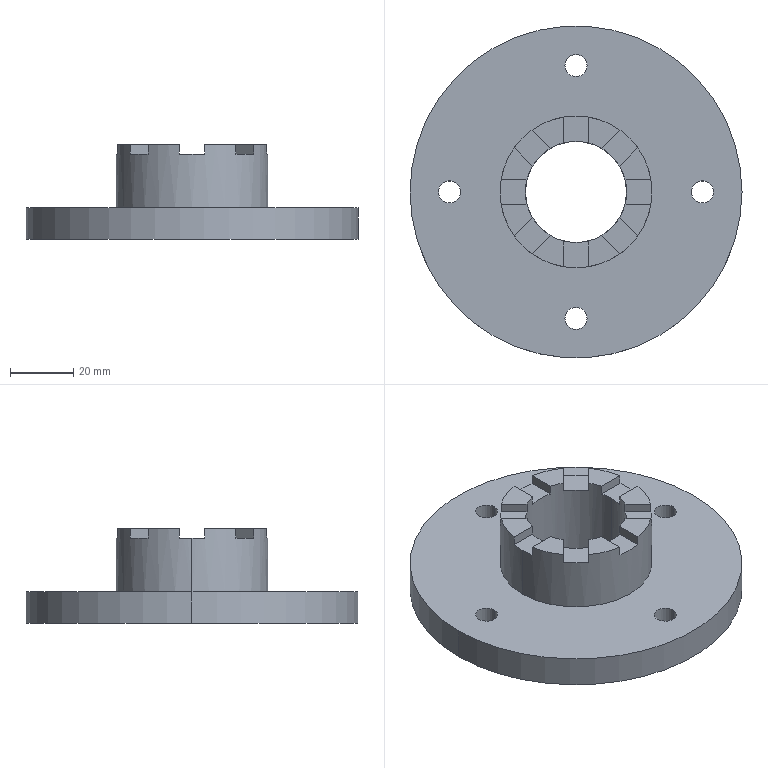Part | SolidWorks | features ICE 2, Extrusion 1 | 1 solid | 48 faces | box 105 x 105 x 30 mm | volume 95568 mm3 | plane 34 | cylinder 14 | commonest cylinder face diameters 7 x8 32 x2 48 x2 105 x2
STEP:
#1=CARTESIAN_POINT('',(24.,0.,27.));
#2=VERTEX_POINT('',#1);
#3=CARTESIAN_POINT('',(23.664,4.,27.));
#4=VERTEX_POINT('',#3);
#5=CARTESIAN_POINT('',(0.,0.,27.));
#6=DIRECTION('',(0.,0.,1.));
#7=DIRECTION('',(1.,0.,0.));
#8=AXIS2_PLACEMENT_3D('',#5,#6,#7);
#9=CIRCLE('',#8,24.);
#10=EDGE_CURVE('',#2,#4,#9,.T.);
#11=ORIENTED_EDGE('',*,*,#10,.F.);
#12=CARTESIAN_POINT('',(24.,0.,10.));
#13=VERTEX_POINT('',#12);
#14=CARTESIAN_POINT('',(24.,0.,30.));
#15=DIRECTION('',(0.,0.,-1.));
#16=VECTOR('',#15,1000.);
#17=LINE('',#14,#16);
#18=EDGE_CURVE('',#2,#13,#17,.T.);
#19=ORIENTED_EDGE('',*,*,#18,.T.);
#20=CARTESIAN_POINT('',(-24.,0.,10.));
#21=VERTEX_POINT('',#20);
#22=CARTESIAN_POINT('',(0.,0.,10.));
#23=DIRECTION('',(0.,0.,1.));
#24=DIRECTION('',(1.,0.,0.));
#25=AXIS2_PLACEMENT_3D('',#22,#23,#24);
#26=CIRCLE('',#25,24.);
#27=EDGE_CURVE('',#13,#21,#26,.T.);
#28=ORIENTED_EDGE('',*,*,#27,.T.);
#29=CARTESIAN_POINT('',(-24.,0.,27.));
#30=VERTEX_POINT('',#29);
#31=CARTESIAN_POINT('',(-24.,0.,30.));
#32=DIRECTION('',(0.,0.,-1.));
#33=VECTOR('',#32,1000.);
#34=LINE('',#31,#33);
#35=EDGE_CURVE('',#30,#21,#34,.T.);
#36=ORIENTED_EDGE('',*,*,#35,.F.);
#37=CARTESIAN_POINT('',(-23.664,4.,27.));
#38=VERTEX_POINT('',#37);
#39=CARTESIAN_POINT('',(0.,0.,27.));
#40=DIRECTION('',(0.,0.,1.));
#41=DIRECTION('',(1.,0.,0.));
#42=AXIS2_PLACEMENT_3D('',#39,#40,#41);
#43=CIRCLE('',#42,24.);
#44=EDGE_CURVE('',#38,#30,#43,.T.);
#45=ORIENTED_EDGE('',*,*,#44,.F.);
#46=CARTESIAN_POINT('',(-23.664,4.,30.));
#47=VERTEX_POINT('',#46);
#48=CARTESIAN_POINT('',(-23.664,4.,27.));
#49=DIRECTION('',(0.,0.,1.));
#50=VECTOR('',#49,1000.);
#51=LINE('',#48,#50);
#52=EDGE_CURVE('',#38,#47,#51,.T.);
#53=ORIENTED_EDGE('',*,*,#52,.T.);
#54=CARTESIAN_POINT('',(-19.562,13.905,30.));
#55=VERTEX_POINT('',#54);
#56=CARTESIAN_POINT('',(0.,0.,30.));
#57=DIRECTION('',(0.,0.,1.));
#58=DIRECTION('',(1.,0.,0.));
#59=AXIS2_PLACEMENT_3D('',#56,#57,#58);
#60=CIRCLE('',#59,24.);
#61=EDGE_CURVE('',#55,#47,#60,.T.);
#62=ORIENTED_EDGE('',*,*,#61,.F.);
#63=CARTESIAN_POINT('',(-19.562,13.905,27.));
#64=VERTEX_POINT('',#63);
#65=CARTESIAN_POINT('',(-19.562,13.905,27.));
#66=DIRECTION('',(0.,0.,1.));
#67=VECTOR('',#66,1000.);
#68=LINE('',#65,#67);
#69=EDGE_CURVE('',#64,#55,#68,.T.);
#70=ORIENTED_EDGE('',*,*,#69,.F.);
#71=CARTESIAN_POINT('',(-13.905,19.562,27.));
#72=VERTEX_POINT('',#71);
#73=CARTESIAN_POINT('',(0.,0.,27.));
#74=DIRECTION('',(0.,0.,1.));
#75=DIRECTION('',(1.,0.,0.));
#76=AXIS2_PLACEMENT_3D('',#73,#74,#75);
#77=CIRCLE('',#76,24.);
#78=EDGE_CURVE('',#72,#64,#77,.T.);
#79=ORIENTED_EDGE('',*,*,#78,.F.);
#80=CARTESIAN_POINT('',(-13.905,19.562,30.));
#81=VERTEX_POINT('',#80);
#82=CARTESIAN_POINT('',(-13.905,19.562,27.));
#83=DIRECTION('',(0.,0.,1.));
#84=VECTOR('',#83,1000.);
#85=LINE('',#82,#84);
#86=EDGE_CURVE('',#72,#81,#85,.T.);
#87=ORIENTED_EDGE('',*,*,#86,.T.);
#88=CARTESIAN_POINT('',(-4.,23.664,30.));
#89=VERTEX_POINT('',#88);
#90=CARTESIAN_POINT('',(0.,0.,30.));
#91=DIRECTION('',(0.,0.,1.));
#92=DIRECTION('',(1.,0.,0.));
#93=AXIS2_PLACEMENT_3D('',#90,#91,#92);
#94=CIRCLE('',#93,24.);
#95=EDGE_CURVE('',#89,#81,#94,.T.);
#96=ORIENTED_EDGE('',*,*,#95,.F.);
#97=CARTESIAN_POINT('',(-4.,23.664,27.));
#98=VERTEX_POINT('',#97);
#99=CARTESIAN_POINT('',(-4.,23.664,27.));
#100=DIRECTION('',(0.,0.,1.));
#101=VECTOR('',#100,1000.);
#102=LINE('',#99,#101);
#103=EDGE_CURVE('',#98,#89,#102,.T.);
#104=ORIENTED_EDGE('',*,*,#103,.F.);
#105=CARTESIAN_POINT('',(4.,23.664,27.));
#106=VERTEX_POINT('',#105);
#107=CARTESIAN_POINT('',(0.,0.,27.));
#108=DIRECTION('',(0.,0.,1.));
#109=DIRECTION('',(1.,0.,0.));
#110=AXIS2_PLACEMENT_3D('',#107,#108,#109);
#111=CIRCLE('',#110,24.);
#112=EDGE_CURVE('',#106,#98,#111,.T.);
#113=ORIENTED_EDGE('',*,*,#112,.F.);
#114=CARTESIAN_POINT('',(4.,23.664,30.));
#115=VERTEX_POINT('',#114);
#116=CARTESIAN_POINT('',(4.,23.664,27.));
#117=DIRECTION('',(0.,0.,1.));
#118=VECTOR('',#117,1000.);
#119=LINE('',#116,#118);
#120=EDGE_CURVE('',#106,#115,#119,.T.);
#121=ORIENTED_EDGE('',*,*,#120,.T.);
#122=CARTESIAN_POINT('',(13.905,19.562,30.));
#123=VERTEX_POINT('',#122);
#124=CARTESIAN_POINT('',(0.,0.,30.));
#125=DIRECTION('',(0.,0.,1.));
#126=DIRECTION('',(1.,0.,0.));
#127=AXIS2_PLACEMENT_3D('',#124,#125,#126);
#128=CIRCLE('',#127,24.);
#129=EDGE_CURVE('',#123,#115,#128,.T.);
#130=ORIENTED_EDGE('',*,*,#129,.F.);
#131=CARTESIAN_POINT('',(13.905,19.562,27.));
#132=VERTEX_POINT('',#131);
#133=CARTESIAN_POINT('',(13.905,19.562,27.));
#134=DIRECTION('',(0.,0.,1.));
#135=VECTOR('',#134,1000.);
#136=LINE('',#133,#135);
#137=EDGE_CURVE('',#132,#123,#136,.T.);
#138=ORIENTED_EDGE('',*,*,#137,.F.);
#139=CARTESIAN_POINT('',(19.562,13.905,27.));
#140=VERTEX_POINT('',#139);
#141=CARTESIAN_POINT('',(0.,0.,27.));
#142=DIRECTION('',(0.,0.,1.));
#143=DIRECTION('',(1.,0.,0.));
#144=AXIS2_PLACEMENT_3D('',#141,#142,#143);
#145=CIRCLE('',#144,24.);
#146=EDGE_CURVE('',#140,#132,#145,.T.);
#147=ORIENTED_EDGE('',*,*,#146,.F.);
#148=CARTESIAN_POINT('',(19.562,13.905,30.));
#149=VERTEX_POINT('',#148);
#150=CARTESIAN_POINT('',(19.562,13.905,27.));
#151=DIRECTION('',(0.,0.,1.));
#152=VECTOR('',#151,1000.);
#153=LINE('',#150,#152);
#154=EDGE_CURVE('',#140,#149,#153,.T.);
#155=ORIENTED_EDGE('',*,*,#154,.T.);
#156=CARTESIAN_POINT('',(23.664,4.,30.));
#157=VERTEX_POINT('',#156);
#158=CARTESIAN_POINT('',(0.,0.,30.));
#159=DIRECTION('',(0.,0.,1.));
#160=DIRECTION('',(1.,0.,0.));
#161=AXIS2_PLACEMENT_3D('',#158,#159,#160);
#162=CIRCLE('',#161,24.);
#163=EDGE_CURVE('',#157,#149,#162,.T.);
#164=ORIENTED_EDGE('',*,*,#163,.F.);
#165=CARTESIAN_POINT('',(23.664,4.,27.));
#166=DIRECTION('',(0.,0.,1.));
#167=VECTOR('',#166,1000.);
#168=LINE('',#165,#167);
#169=EDGE_CURVE('',#4,#157,#168,.T.);
#170=ORIENTED_EDGE('',*,*,#169,.F.);
#171=EDGE_LOOP('',(#11,#19,#28,#36,#45,#53,#62,#70,#79,#87,#96,#104,#113,#121,#130,#138,#147,#155,#164,#170));
#172=FACE_OUTER_BOUND('',#171,.T.);
#173=CARTESIAN_POINT('',(0.,0.,30.));
#174=DIRECTION('',(0.,0.,-1.));
#175=DIRECTION('',(-1.,0.,0.));
#176=AXIS2_PLACEMENT_3D('',#173,#174,#175);
#177=CYLINDRICAL_SURFACE('',#176,24.);
#178=ADVANCED_FACE('',(#172),#177,.T.);
#179=CARTESIAN_POINT('',(16.,0.,27.));
#180=VERTEX_POINT('',#179);
#181=CARTESIAN_POINT('',(15.492,-4.,27.));
#182=VERTEX_POINT('',#181);
#183=CARTESIAN_POINT('',(0.,0.,27.));
#184=DIRECTION('',(0.,0.,-1.));
#185=DIRECTION('',(1.,0.,0.));
#186=AXIS2_PLACEMENT_3D('',#183,#184,#185);
#187=CIRCLE('',#186,16.);
#188=EDGE_CURVE('',#180,#182,#187,.T.);
#189=ORIENTED_EDGE('',*,*,#188,.F.);
#190=CARTESIAN_POINT('',(16.,0.,0.));
#191=VERTEX_POINT('',#190);
#192=CARTESIAN_POINT('',(16.,0.,10.));
#193=DIRECTION('',(0.,0.,-1.));
#194=VECTOR('',#193,1000.);
#195=LINE('',#192,#194);
#196=EDGE_CURVE('',#180,#191,#195,.T.);
#197=ORIENTED_EDGE('',*,*,#196,.T.);
#198=CARTESIAN_POINT('',(-16.,0.,0.));
#199=VERTEX_POINT('',#198);
#200=CARTESIAN_POINT('',(0.,0.,0.));
#201=DIRECTION('',(0.,0.,1.));
#202=DIRECTION('',(1.,0.,0.));
#203=AXIS2_PLACEMENT_3D('',#200,#201,#202);
#204=CIRCLE('',#203,16.);
#205=EDGE_CURVE('',#199,#191,#204,.T.);
#206=ORIENTED_EDGE('',*,*,#205,.F.);
#207=CARTESIAN_POINT('',(-16.,0.,27.));
#208=VERTEX_POINT('',#207);
#209=CARTESIAN_POINT('',(-16.,0.,10.));
#210=DIRECTION('',(0.,0.,-1.));
#211=VECTOR('',#210,1000.);
#212=LINE('',#209,#211);
#213=EDGE_CURVE('',#208,#199,#212,.T.);
#214=ORIENTED_EDGE('',*,*,#213,.F.);
#215=CARTESIAN_POINT('',(-15.492,-4.,27.));
#216=VERTEX_POINT('',#215);
#217=CARTESIAN_POINT('',(0.,0.,27.));
#218=DIRECTION('',(0.,0.,-1.));
#219=DIRECTION('',(1.,0.,0.));
#220=AXIS2_PLACEMENT_3D('',#217,#218,#219);
#221=CIRCLE('',#220,16.);
#222=EDGE_CURVE('',#216,#208,#221,.T.);
#223=ORIENTED_EDGE('',*,*,#222,.F.);
#224=CARTESIAN_POINT('',(-15.492,-4.,30.));
#225=VERTEX_POINT('',#224);
#226=CARTESIAN_POINT('',(-15.492,-4.,27.));
#227=DIRECTION('',(0.,0.,1.));
#228=VECTOR('',#227,1000.);
#229=LINE('',#226,#228);
#230=EDGE_CURVE('',#216,#225,#229,.T.);
#231=ORIENTED_EDGE('',*,*,#230,.T.);
#232=CARTESIAN_POINT('',(-13.783,-8.126,30.));
#233=VERTEX_POINT('',#232);
#234=CARTESIAN_POINT('',(0.,0.,30.));
#235=DIRECTION('',(0.,0.,1.));
#236=DIRECTION('',(1.,0.,0.));
#237=AXIS2_PLACEMENT_3D('',#234,#235,#236);
#238=CIRCLE('',#237,16.);
#239=EDGE_CURVE('',#225,#233,#238,.T.);
#240=ORIENTED_EDGE('',*,*,#239,.T.);
#241=CARTESIAN_POINT('',(-13.783,-8.126,27.));
#242=VERTEX_POINT('',#241);
#243=CARTESIAN_POINT('',(-13.783,-8.126,27.));
#244=DIRECTION('',(0.,0.,1.));
#245=VECTOR('',#244,1000.);
#246=LINE('',#243,#245);
#247=EDGE_CURVE('',#242,#233,#246,.T.);
#248=ORIENTED_EDGE('',*,*,#247,.F.);
#249=CARTESIAN_POINT('',(-8.126,-13.783,27.));
#250=VERTEX_POINT('',#249);
#251=CARTESIAN_POINT('',(0.,0.,27.));
#252=DIRECTION('',(0.,0.,-1.));
#253=DIRECTION('',(1.,0.,0.));
#254=AXIS2_PLACEMENT_3D('',#251,#252,#253);
#255=CIRCLE('',#254,16.);
#256=EDGE_CURVE('',#250,#242,#255,.T.);
#257=ORIENTED_EDGE('',*,*,#256,.F.);
#258=CARTESIAN_POINT('',(-8.126,-13.783,30.));
#259=VERTEX_POINT('',#258);
#260=CARTESIAN_POINT('',(-8.126,-13.783,27.));
#261=DIRECTION('',(0.,0.,1.));
#262=VECTOR('',#261,1000.);
#263=LINE('',#260,#262);
#264=EDGE_CURVE('',#250,#259,#263,.T.);
#265=ORIENTED_EDGE('',*,*,#264,.T.);
#266=CARTESIAN_POINT('',(-4.,-15.492,30.));
#267=VERTEX_POINT('',#266);
#268=CARTESIAN_POINT('',(0.,0.,30.));
#269=DIRECTION('',(0.,0.,1.));
#270=DIRECTION('',(1.,0.,0.));
#271=AXIS2_PLACEMENT_3D('',#268,#269,#270);
#272=CIRCLE('',#271,16.);
#273=EDGE_CURVE('',#259,#267,#272,.T.);
#274=ORIENTED_EDGE('',*,*,#273,.T.);
#275=CARTESIAN_POINT('',(-4.,-15.492,27.));
#276=VERTEX_POINT('',#275);
#277=CARTESIAN_POINT('',(-4.,-15.492,27.));
#278=DIRECTION('',(0.,0.,1.));
#279=VECTOR('',#278,1000.);
#280=LINE('',#277,#279);
#281=EDGE_CURVE('',#276,#267,#280,.T.);
#282=ORIENTED_EDGE('',*,*,#281,.F.);
#283=CARTESIAN_POINT('',(4.,-15.492,27.));
#284=VERTEX_POINT('',#283);
#285=CARTESIAN_POINT('',(0.,0.,27.));
#286=DIRECTION('',(0.,0.,-1.));
#287=DIRECTION('',(1.,0.,0.));
#288=AXIS2_PLACEMENT_3D('',#285,#286,#287);
#289=CIRCLE('',#288,16.);
#290=EDGE_CURVE('',#284,#276,#289,.T.);
#291=ORIENTED_EDGE('',*,*,#290,.F.);
#292=CARTESIAN_POINT('',(4.,-15.492,30.));
#293=VERTEX_POINT('',#292);
#294=CARTESIAN_POINT('',(4.,-15.492,27.));
#295=DIRECTION('',(0.,0.,1.));
#296=VECTOR('',#295,1000.);
#297=LINE('',#294,#296);
#298=EDGE_CURVE('',#284,#293,#297,.T.);
#299=ORIENTED_EDGE('',*,*,#298,.T.);
#300=CARTESIAN_POINT('',(8.126,-13.783,30.));
#301=VERTEX_POINT('',#300);
#302=CARTESIAN_POINT('',(0.,0.,30.));
#303=DIRECTION('',(0.,0.,1.));
#304=DIRECTION('',(1.,0.,0.));
#305=AXIS2_PLACEMENT_3D('',#302,#303,#304);
#306=CIRCLE('',#305,16.);
#307=EDGE_CURVE('',#293,#301,#306,.T.);
#308=ORIENTED_EDGE('',*,*,#307,.T.);
#309=CARTESIAN_POINT('',(8.126,-13.783,27.));
#310=VERTEX_POINT('',#309);
#311=CARTESIAN_POINT('',(8.126,-13.783,27.));
#312=DIRECTION('',(0.,0.,1.));
#313=VECTOR('',#312,1000.);
#314=LINE('',#311,#313);
#315=EDGE_CURVE('',#310,#301,#314,.T.);
#316=ORIENTED_EDGE('',*,*,#315,.F.);
#317=CARTESIAN_POINT('',(13.783,-8.126,27.));
#318=VERTEX_POINT('',#317);
#319=CARTESIAN_POINT('',(0.,0.,27.));
#320=DIRECTION('',(0.,0.,-1.));
#321=DIRECTION('',(1.,0.,0.));
#322=AXIS2_PLACEMENT_3D('',#319,#320,#321);
#323=CIRCLE('',#322,16.);
#324=EDGE_CURVE('',#318,#310,#323,.T.);
#325=ORIENTED_EDGE('',*,*,#324,.F.);
#326=CARTESIAN_POINT('',(13.783,-8.126,30.));
#327=VERTEX_POINT('',#326);
#328=CARTESIAN_POINT('',(13.783,-8.126,27.));
#329=DIRECTION('',(0.,0.,1.));
#330=VECTOR('',#329,1000.);
#331=LINE('',#328,#330);
#332=EDGE_CURVE('',#318,#327,#331,.T.);
#333=ORIENTED_EDGE('',*,*,#332,.T.);
#334=CARTESIAN_POINT('',(15.492,-4.,30.));
#335=VERTEX_POINT('',#334);
#336=CARTESIAN_POINT('',(0.,0.,30.));
#337=DIRECTION('',(0.,0.,1.));
#338=DIRECTION('',(1.,0.,0.));
#339=AXIS2_PLACEMENT_3D('',#336,#337,#338);
#340=CIRCLE('',#339,16.);
#341=EDGE_CURVE('',#327,#335,#340,.T.);
#342=ORIENTED_EDGE('',*,*,#341,.T.);
#343=CARTESIAN_POINT('',(15.492,-4.,27.));
#344=DIRECTION('',(0.,0.,1.));
#345=VECTOR('',#344,1000.);
#346=LINE('',#343,#345);
#347=EDGE_CURVE('',#182,#335,#346,.T.);
#348=ORIENTED_EDGE('',*,*,#347,.F.);
#349=EDGE_LOOP('',(#189,#197,#206,#214,#223,#231,#240,#248,#257,#265,#274,#282,#291,#299,#308,#316,#325,#333,#342,#348));
#350=FACE_OUTER_BOUND('',#349,.T.);
#351=CARTESIAN_POINT('',(0.,0.,10.));
#352=DIRECTION('',(0.,0.,-1.));
#353=DIRECTION('',(-1.,0.,0.));
#354=AXIS2_PLACEMENT_3D('',#351,#352,#353);
#355=CYLINDRICAL_SURFACE('',#354,16.);
#356=ADVANCED_FACE('',(#350),#355,.F.);
#357=CARTESIAN_POINT('',(-43.5,0.,10.));
#358=VERTEX_POINT('',#357);
#359=CARTESIAN_POINT('',(-36.5,0.,10.));
#360=VERTEX_POINT('',#359);
#361=CARTESIAN_POINT('',(-40.,0.,10.));
#362=DIRECTION('',(0.,0.,1.));
#363=DIRECTION('',(1.,0.,0.));
#364=AXIS2_PLACEMENT_3D('',#361,#362,#363);
#365=CIRCLE('',#364,3.5);
#366=EDGE_CURVE('',#358,#360,#365,.T.);
#367=ORIENTED_EDGE('',*,*,#366,.T.);
#368=CARTESIAN_POINT('',(-36.5,0.,0.));
#369=VERTEX_POINT('',#368);
#370=CARTESIAN_POINT('',(-36.5,0.,10.));
#371=DIRECTION('',(0.,0.,-1.));
#372=VECTOR('',#371,1000.);
#373=LINE('',#370,#372);
#374=EDGE_CURVE('',#360,#369,#373,.T.);
#375=ORIENTED_EDGE('',*,*,#374,.T.);
#376=CARTESIAN_POINT('',(-43.5,0.,0.));
#377=VERTEX_POINT('',#376);
#378=CARTESIAN_POINT('',(-40.,0.,0.));
#379=DIRECTION('',(0.,0.,1.));
#380=DIRECTION('',(1.,0.,0.));
#381=AXIS2_PLACEMENT_3D('',#378,#379,#380);
#382=CIRCLE('',#381,3.5);
#383=EDGE_CURVE('',#377,#369,#382,.T.);
#384=ORIENTED_EDGE('',*,*,#383,.F.);
#385=CARTESIAN_POINT('',(-43.5,0.,10.));
#386=DIRECTION('',(0.,0.,-1.));
#387=VECTOR('',#386,1000.);
#388=LINE('',#385,#387);
#389=EDGE_CURVE('',#358,#377,#388,.T.);
#390=ORIENTED_EDGE('',*,*,#389,.F.);
#391=EDGE_LOOP('',(#367,#375,#384,#390));
#392=FACE_OUTER_BOUND('',#391,.T.);
#393=CARTESIAN_POINT('',(-40.,0.,10.));
#394=DIRECTION('',(0.,0.,-1.));
#395=DIRECTION('',(-1.,0.,0.));
#396=AXIS2_PLACEMENT_3D('',#393,#394,#395);
#397=CYLINDRICAL_SURFACE('',#396,3.5);
#398=ADVANCED_FACE('',(#392),#397,.F.);
#399=CARTESIAN_POINT('',(-3.5,-40.,10.));
#400=VERTEX_POINT('',#399);
#401=CARTESIAN_POINT('',(3.5,-40.,10.));
#402=VERTEX_POINT('',#401);
#403=CARTESIAN_POINT('',(0.,-40.,10.));
#404=DIRECTION('',(0.,0.,1.));
#405=DIRECTION('',(1.,0.,0.));
#406=AXIS2_PLACEMENT_3D('',#403,#404,#405);
#407=CIRCLE('',#406,3.5);
#408=EDGE_CURVE('',#400,#402,#407,.T.);
#409=ORIENTED_EDGE('',*,*,#408,.T.);
#410=CARTESIAN_POINT('',(3.5,-40.,0.));
#411=VERTEX_POINT('',#410);
#412=CARTESIAN_POINT('',(3.5,-40.,10.));
#413=DIRECTION('',(0.,0.,-1.));
#414=VECTOR('',#413,1000.);
#415=LINE('',#412,#414);
#416=EDGE_CURVE('',#402,#411,#415,.T.);
#417=ORIENTED_EDGE('',*,*,#416,.T.);
#418=CARTESIAN_POINT('',(-3.5,-40.,0.));
#419=VERTEX_POINT('',#418);
#420=CARTESIAN_POINT('',(0.,-40.,0.));
#421=DIRECTION('',(0.,0.,1.));
#422=DIRECTION('',(1.,0.,0.));
#423=AXIS2_PLACEMENT_3D('',#420,#421,#422);
#424=CIRCLE('',#423,3.5);
#425=EDGE_CURVE('',#419,#411,#424,.T.);
#426=ORIENTED_EDGE('',*,*,#425,.F.);
#427=CARTESIAN_POINT('',(-3.5,-40.,10.));
#428=DIRECTION('',(0.,0.,-1.));
#429=VECTOR('',#428,1000.);
#430=LINE('',#427,#429);
#431=EDGE_CURVE('',#400,#419,#430,.T.);
#432=ORIENTED_EDGE('',*,*,#431,.F.);
#433=EDGE_LOOP('',(#409,#417,#426,#432));
#434=FACE_OUTER_BOUND('',#433,.T.);
#435=CARTESIAN_POINT('',(0.,-40.,10.));
#436=DIRECTION('',(0.,0.,-1.));
#437=DIRECTION('',(-1.,0.,0.));
#438=AXIS2_PLACEMENT_3D('',#435,#436,#437);
#439=CYLINDRICAL_SURFACE('',#438,3.5);
#440=ADVANCED_FACE('',(#434),#439,.F.);
#441=CARTESIAN_POINT('',(36.5,0.,10.));
#442=VERTEX_POINT('',#441);
#443=CARTESIAN_POINT('',(43.5,0.,10.));
#444=VERTEX_POINT('',#443);
#445=CARTESIAN_POINT('',(40.,0.,10.));
#446=DIRECTION('',(0.,0.,1.));
#447=DIRECTION('',(1.,0.,0.));
#448=AXIS2_PLACEMENT_3D('',#445,#446,#447);
#449=CIRCLE('',#448,3.5);
#450=EDGE_CURVE('',#442,#444,#449,.T.);
#451=ORIENTED_EDGE('',*,*,#450,.T.);
#452=CARTESIAN_POINT('',(43.5,0.,0.));
#453=VERTEX_POINT('',#452);
#454=CARTESIAN_POINT('',(43.5,0.,10.));
#455=DIRECTION('',(0.,0.,-1.));
#456=VECTOR('',#455,1000.);
#457=LINE('',#454,#456);
#458=EDGE_CURVE('',#444,#453,#457,.T.);
#459=ORIENTED_EDGE('',*,*,#458,.T.);
#460=CARTESIAN_POINT('',(36.5,0.,0.));
#461=VERTEX_POINT('',#460);
#462=CARTESIAN_POINT('',(40.,0.,0.));
#463=DIRECTION('',(0.,0.,1.));
#464=DIRECTION('',(1.,0.,0.));
#465=AXIS2_PLACEMENT_3D('',#462,#463,#464);
#466=CIRCLE('',#465,3.5);
#467=EDGE_CURVE('',#461,#453,#466,.T.);
#468=ORIENTED_EDGE('',*,*,#467,.F.);
#469=CARTESIAN_POINT('',(36.5,0.,10.));
#470=DIRECTION('',(0.,0.,-1.));
#471=VECTOR('',#470,1000.);
#472=LINE('',#469,#471);
#473=EDGE_CURVE('',#442,#461,#472,.T.);
#474=ORIENTED_EDGE('',*,*,#473,.F.);
#475=EDGE_LOOP('',(#451,#459,#468,#474));
#476=FACE_OUTER_BOUND('',#475,.T.);
#477=CARTESIAN_POINT('',(40.,0.,10.));
#478=DIRECTION('',(0.,0.,-1.));
#479=DIRECTION('',(-1.,0.,0.));
#480=AXIS2_PLACEMENT_3D('',#477,#478,#479);
#481=CYLINDRICAL_SURFACE('',#480,3.5);
#482=ADVANCED_FACE('',(#476),#481,.F.);
#483=CARTESIAN_POINT('',(-3.5,40.,10.));
#484=VERTEX_POINT('',#483);
#485=CARTESIAN_POINT('',(3.5,40.,10.));
#486=VERTEX_POINT('',#485);
#487=CARTESIAN_POINT('',(0.,40.,10.));
#488=DIRECTION('',(0.,0.,1.));
#489=DIRECTION('',(1.,0.,0.));
#490=AXIS2_PLACEMENT_3D('',#487,#488,#489);
#491=CIRCLE('',#490,3.5);
#492=EDGE_CURVE('',#484,#486,#491,.T.);
#493=ORIENTED_EDGE('',*,*,#492,.T.);
#494=CARTESIAN_POINT('',(3.5,40.,0.));
#495=VERTEX_POINT('',#494);
#496=CARTESIAN_POINT('',(3.5,40.,10.));
#497=DIRECTION('',(0.,0.,-1.));
#498=VECTOR('',#497,1000.);
#499=LINE('',#496,#498);
#500=EDGE_CURVE('',#486,#495,#499,.T.);
#501=ORIENTED_EDGE('',*,*,#500,.T.);
#502=CARTESIAN_POINT('',(-3.5,40.,0.));
#503=VERTEX_POINT('',#502);
#504=CARTESIAN_POINT('',(0.,40.,0.));
#505=DIRECTION('',(0.,0.,1.));
#506=DIRECTION('',(1.,0.,0.));
#507=AXIS2_PLACEMENT_3D('',#504,#505,#506);
#508=CIRCLE('',#507,3.5);
#509=EDGE_CURVE('',#503,#495,#508,.T.);
#510=ORIENTED_EDGE('',*,*,#509,.F.);
#511=CARTESIAN_POINT('',(-3.5,40.,10.));
#512=DIRECTION('',(0.,0.,-1.));
#513=VECTOR('',#512,1000.);
#514=LINE('',#511,#513);
#515=EDGE_CURVE('',#484,#503,#514,.T.);
#516=ORIENTED_EDGE('',*,*,#515,.F.);
#517=EDGE_LOOP('',(#493,#501,#510,#516));
#518=FACE_OUTER_BOUND('',#517,.T.);
#519=CARTESIAN_POINT('',(0.,40.,10.));
#520=DIRECTION('',(0.,0.,-1.));
#521=DIRECTION('',(-1.,0.,0.));
#522=AXIS2_PLACEMENT_3D('',#519,#520,#521);
#523=CYLINDRICAL_SURFACE('',#522,3.5);
#524=ADVANCED_FACE('',(#518),#523,.F.);
#525=CARTESIAN_POINT('',(52.5,0.,10.));
#526=VERTEX_POINT('',#525);
#527=CARTESIAN_POINT('',(-52.5,0.,10.));
#528=VERTEX_POINT('',#527);
#529=CARTESIAN_POINT('',(0.,0.,10.));
#530=DIRECTION('',(0.,0.,1.));
#531=DIRECTION('',(1.,0.,0.));
#532=AXIS2_PLACEMENT_3D('',#529,#530,#531);
#533=CIRCLE('',#532,52.5);
#534=EDGE_CURVE('',#526,#528,#533,.T.);
#535=ORIENTED_EDGE('',*,*,#534,.F.);
#536=CARTESIAN_POINT('',(52.5,0.,0.));
#537=VERTEX_POINT('',#536);
#538=CARTESIAN_POINT('',(52.5,0.,10.));
#539=DIRECTION('',(0.,0.,-1.));
#540=VECTOR('',#539,1000.);
#541=LINE('',#538,#540);
#542=EDGE_CURVE('',#526,#537,#541,.T.);
#543=ORIENTED_EDGE('',*,*,#542,.T.);
#544=CARTESIAN_POINT('',(-52.5,0.,0.));
#545=VERTEX_POINT('',#544);
#546=CARTESIAN_POINT('',(0.,0.,0.));
#547=DIRECTION('',(0.,0.,1.));
#548=DIRECTION('',(1.,0.,0.));
#549=AXIS2_PLACEMENT_3D('',#546,#547,#548);
#550=CIRCLE('',#549,52.5);
#551=EDGE_CURVE('',#537,#545,#550,.T.);
#552=ORIENTED_EDGE('',*,*,#551,.T.);
#553=CARTESIAN_POINT('',(-52.5,0.,10.));
#554=DIRECTION('',(0.,0.,-1.));
#555=VECTOR('',#554,1000.);
#556=LINE('',#553,#555);
#557=EDGE_CURVE('',#528,#545,#556,.T.);
#558=ORIENTED_EDGE('',*,*,#557,.F.);
#559=EDGE_LOOP('',(#535,#543,#552,#558));
#560=FACE_OUTER_BOUND('',#559,.T.);
#561=CARTESIAN_POINT('',(0.,0.,10.));
#562=DIRECTION('',(0.,0.,-1.));
#563=DIRECTION('',(-1.,0.,0.));
#564=AXIS2_PLACEMENT_3D('',#561,#562,#563);
#565=CYLINDRICAL_SURFACE('',#564,52.5);
#566=ADVANCED_FACE('',(#560),#565,.T.);
#567=CARTESIAN_POINT('',(-8.126,13.783,30.));
#568=VERTEX_POINT('',#567);
#569=CARTESIAN_POINT('',(-13.905,19.562,30.));
#570=DIRECTION('',(-0.7071,0.7071,0.));
#571=VECTOR('',#570,1000.);
#572=LINE('',#569,#571);
#573=EDGE_CURVE('',#568,#81,#572,.T.);
#574=ORIENTED_EDGE('',*,*,#573,.F.);
#575=CARTESIAN_POINT('',(-4.,15.492,30.));
#576=VERTEX_POINT('',#575);
#577=CARTESIAN_POINT('',(0.,0.,30.));
#578=DIRECTION('',(0.,0.,1.));
#579=DIRECTION('',(1.,0.,0.));
#580=AXIS2_PLACEMENT_3D('',#577,#578,#579);
#581=CIRCLE('',#580,16.);
#582=EDGE_CURVE('',#576,#568,#581,.T.);
#583=ORIENTED_EDGE('',*,*,#582,.F.);
#584=CARTESIAN_POINT('',(-4.,23.664,30.));
#585=DIRECTION('',(0.,-1.,0.));
#586=VECTOR('',#585,1000.);
#587=LINE('',#584,#586);
#588=EDGE_CURVE('',#89,#576,#587,.T.);
#589=ORIENTED_EDGE('',*,*,#588,.F.);
#590=ORIENTED_EDGE('',*,*,#95,.T.);
#591=EDGE_LOOP('',(#574,#583,#589,#590));
#592=FACE_OUTER_BOUND('',#591,.T.);
#593=CARTESIAN_POINT('',(0.,0.,30.));
#594=DIRECTION('',(0.,0.,1.));
#595=DIRECTION('',(1.,0.,0.));
#596=AXIS2_PLACEMENT_3D('',#593,#594,#595);
#597=PLANE('',#596);
#598=ADVANCED_FACE('',(#592),#597,.T.);
#599=CARTESIAN_POINT('',(-13.783,8.126,30.));
#600=VERTEX_POINT('',#599);
#601=CARTESIAN_POINT('',(-19.562,13.905,30.));
#602=DIRECTION('',(0.7071,-0.7071,0.));
#603=VECTOR('',#602,1000.);
#604=LINE('',#601,#603);
#605=EDGE_CURVE('',#55,#600,#604,.T.);
#606=ORIENTED_EDGE('',*,*,#605,.F.);
#607=ORIENTED_EDGE('',*,*,#61,.T.);
#608=CARTESIAN_POINT('',(-15.492,4.,30.));
#609=VERTEX_POINT('',#608);
#610=CARTESIAN_POINT('',(-23.664,4.,30.));
#611=DIRECTION('',(-1.,0.,0.));
#612=VECTOR('',#611,1000.);
#613=LINE('',#610,#612);
#614=EDGE_CURVE('',#609,#47,#613,.T.);
#615=ORIENTED_EDGE('',*,*,#614,.F.);
#616=CARTESIAN_POINT('',(0.,0.,30.));
#617=DIRECTION('',(0.,0.,1.));
#618=DIRECTION('',(1.,0.,0.));
#619=AXIS2_PLACEMENT_3D('',#616,#617,#618);
#620=CIRCLE('',#619,16.);
#621=EDGE_CURVE('',#600,#609,#620,.T.);
#622=ORIENTED_EDGE('',*,*,#621,.F.);
#623=EDGE_LOOP('',(#606,#607,#615,#622));
#624=FACE_OUTER_BOUND('',#623,.T.);
#625=CARTESIAN_POINT('',(0.,0.,30.));
#626=DIRECTION('',(0.,0.,1.));
#627=DIRECTION('',(1.,0.,0.));
#628=AXIS2_PLACEMENT_3D('',#625,#626,#627);
#629=PLANE('',#628);
#630=ADVANCED_FACE('',(#624),#629,.T.);
#631=CARTESIAN_POINT('',(-23.664,-4.,30.));
#632=VERTEX_POINT('',#631);
#633=CARTESIAN_POINT('',(-23.664,-4.,30.));
#634=DIRECTION('',(1.,0.,0.));
#635=VECTOR('',#634,1000.);
#636=LINE('',#633,#635);
#637=EDGE_CURVE('',#632,#225,#636,.T.);
#638=ORIENTED_EDGE('',*,*,#637,.F.);
#639=CARTESIAN_POINT('',(-19.562,-13.905,30.));
#640=VERTEX_POINT('',#639);
#641=CARTESIAN_POINT('',(0.,0.,30.));
#642=DIRECTION('',(0.,0.,1.));
#643=DIRECTION('',(1.,0.,0.));
#644=AXIS2_PLACEMENT_3D('',#641,#642,#643);
#645=CIRCLE('',#644,24.);
#646=EDGE_CURVE('',#632,#640,#645,.T.);
#647=ORIENTED_EDGE('',*,*,#646,.T.);
#648=CARTESIAN_POINT('',(-19.562,-13.905,30.));
#649=DIRECTION('',(-0.7071,-0.7071,0.));
#650=VECTOR('',#649,1000.);
#651=LINE('',#648,#650);
#652=EDGE_CURVE('',#233,#640,#651,.T.);
#653=ORIENTED_EDGE('',*,*,#652,.F.);
#654=ORIENTED_EDGE('',*,*,#239,.F.);
#655=EDGE_LOOP('',(#638,#647,#653,#654));
#656=FACE_OUTER_BOUND('',#655,.T.);
#657=CARTESIAN_POINT('',(0.,0.,30.));
#658=DIRECTION('',(0.,0.,1.));
#659=DIRECTION('',(1.,0.,0.));
#660=AXIS2_PLACEMENT_3D('',#657,#658,#659);
#661=PLANE('',#660);
#662=ADVANCED_FACE('',(#656),#661,.T.);
#663=CARTESIAN_POINT('',(-13.905,-19.562,30.));
#664=VERTEX_POINT('',#663);
#665=CARTESIAN_POINT('',(-13.905,-19.562,30.));
#666=DIRECTION('',(0.7071,0.7071,0.));
#667=VECTOR('',#666,1000.);
#668=LINE('',#665,#667);
#669=EDGE_CURVE('',#664,#259,#668,.T.);
#670=ORIENTED_EDGE('',*,*,#669,.F.);
#671=CARTESIAN_POINT('',(-4.,-23.664,30.));
#672=VERTEX_POINT('',#671);
#673=CARTESIAN_POINT('',(0.,0.,30.));
#674=DIRECTION('',(0.,0.,1.));
#675=DIRECTION('',(1.,0.,0.));
#676=AXIS2_PLACEMENT_3D('',#673,#674,#675);
#677=CIRCLE('',#676,24.);
#678=EDGE_CURVE('',#664,#672,#677,.T.);
#679=ORIENTED_EDGE('',*,*,#678,.T.);
#680=CARTESIAN_POINT('',(-4.,-23.664,30.));
#681=DIRECTION('',(0.,-1.,0.));
#682=VECTOR('',#681,1000.);
#683=LINE('',#680,#682);
#684=EDGE_CURVE('',#267,#672,#683,.T.);
#685=ORIENTED_EDGE('',*,*,#684,.F.);
#686=ORIENTED_EDGE('',*,*,#273,.F.);
#687=EDGE_LOOP('',(#670,#679,#685,#686));
#688=FACE_OUTER_BOUND('',#687,.T.);
#689=CARTESIAN_POINT('',(0.,0.,30.));
#690=DIRECTION('',(0.,0.,1.));
#691=DIRECTION('',(1.,0.,0.));
#692=AXIS2_PLACEMENT_3D('',#689,#690,#691);
#693=PLANE('',#692);
#694=ADVANCED_FACE('',(#688),#693,.T.);
#695=CARTESIAN_POINT('',(4.,-23.664,30.));
#696=VERTEX_POINT('',#695);
#697=CARTESIAN_POINT('',(4.,-23.664,30.));
#698=DIRECTION('',(0.,1.,0.));
#699=VECTOR('',#698,1000.);
#700=LINE('',#697,#699);
#701=EDGE_CURVE('',#696,#293,#700,.T.);
#702=ORIENTED_EDGE('',*,*,#701,.F.);
#703=CARTESIAN_POINT('',(13.905,-19.562,30.));
#704=VERTEX_POINT('',#703);
#705=CARTESIAN_POINT('',(0.,0.,30.));
#706=DIRECTION('',(0.,0.,1.));
#707=DIRECTION('',(1.,0.,0.));
#708=AXIS2_PLACEMENT_3D('',#705,#706,#707);
#709=CIRCLE('',#708,24.);
#710=EDGE_CURVE('',#696,#704,#709,.T.);
#711=ORIENTED_EDGE('',*,*,#710,.T.);
#712=CARTESIAN_POINT('',(13.905,-19.562,30.));
#713=DIRECTION('',(0.7071,-0.7071,0.));
#714=VECTOR('',#713,1000.);
#715=LINE('',#712,#714);
#716=EDGE_CURVE('',#301,#704,#715,.T.);
#717=ORIENTED_EDGE('',*,*,#716,.F.);
#718=ORIENTED_EDGE('',*,*,#307,.F.);
#719=EDGE_LOOP('',(#702,#711,#717,#718));
#720=FACE_OUTER_BOUND('',#719,.T.);
#721=CARTESIAN_POINT('',(0.,0.,30.));
#722=DIRECTION('',(0.,0.,1.));
#723=DIRECTION('',(1.,0.,0.));
#724=AXIS2_PLACEMENT_3D('',#721,#722,#723);
#725=PLANE('',#724);
#726=ADVANCED_FACE('',(#720),#725,.T.);
#727=CARTESIAN_POINT('',(19.562,-13.905,30.));
#728=VERTEX_POINT('',#727);
#729=CARTESIAN_POINT('',(19.562,-13.905,30.));
#730=DIRECTION('',(-0.7071,0.7071,0.));
#731=VECTOR('',#730,1000.);
#732=LINE('',#729,#731);
#733=EDGE_CURVE('',#728,#327,#732,.T.);
#734=ORIENTED_EDGE('',*,*,#733,.F.);
#735=CARTESIAN_POINT('',(23.664,-4.,30.));
#736=VERTEX_POINT('',#735);
#737=CARTESIAN_POINT('',(0.,0.,30.));
#738=DIRECTION('',(0.,0.,1.));
#739=DIRECTION('',(1.,0.,0.));
#740=AXIS2_PLACEMENT_3D('',#737,#738,#739);
#741=CIRCLE('',#740,24.);
#742=EDGE_CURVE('',#728,#736,#741,.T.);
#743=ORIENTED_EDGE('',*,*,#742,.T.);
#744=CARTESIAN_POINT('',(23.664,-4.,30.));
#745=DIRECTION('',(1.,0.,0.));
#746=VECTOR('',#745,1000.);
#747=LINE('',#744,#746);
#748=EDGE_CURVE('',#335,#736,#747,.T.);
#749=ORIENTED_EDGE('',*,*,#748,.F.);
#750=ORIENTED_EDGE('',*,*,#341,.F.);
#751=EDGE_LOOP('',(#734,#743,#749,#750));
#752=FACE_OUTER_BOUND('',#751,.T.);
#753=CARTESIAN_POINT('',(0.,0.,30.));
#754=DIRECTION('',(0.,0.,1.));
#755=DIRECTION('',(1.,0.,0.));
#756=AXIS2_PLACEMENT_3D('',#753,#754,#755);
#757=PLANE('',#756);
#758=ADVANCED_FACE('',(#752),#757,.T.);
#759=CARTESIAN_POINT('',(15.492,4.,30.));
#760=VERTEX_POINT('',#759);
#761=CARTESIAN_POINT('',(23.664,4.,30.));
#762=DIRECTION('',(-1.,0.,0.));
#763=VECTOR('',#762,1000.);
#764=LINE('',#761,#763);
#765=EDGE_CURVE('',#157,#760,#764,.T.);
#766=ORIENTED_EDGE('',*,*,#765,.F.);
#767=ORIENTED_EDGE('',*,*,#163,.T.);
#768=CARTESIAN_POINT('',(13.783,8.126,30.));
#769=VERTEX_POINT('',#768);
#770=CARTESIAN_POINT('',(19.562,13.905,30.));
#771=DIRECTION('',(0.7071,0.7071,0.));
#772=VECTOR('',#771,1000.);
#773=LINE('',#770,#772);
#774=EDGE_CURVE('',#769,#149,#773,.T.);
#775=ORIENTED_EDGE('',*,*,#774,.F.);
#776=CARTESIAN_POINT('',(0.,0.,30.));
#777=DIRECTION('',(0.,0.,1.));
#778=DIRECTION('',(1.,0.,0.));
#779=AXIS2_PLACEMENT_3D('',#776,#777,#778);
#780=CIRCLE('',#779,16.);
#781=EDGE_CURVE('',#760,#769,#780,.T.);
#782=ORIENTED_EDGE('',*,*,#781,.F.);
#783=EDGE_LOOP('',(#766,#767,#775,#782));
#784=FACE_OUTER_BOUND('',#783,.T.);
#785=CARTESIAN_POINT('',(0.,0.,30.));
#786=DIRECTION('',(0.,0.,1.));
#787=DIRECTION('',(1.,0.,0.));
#788=AXIS2_PLACEMENT_3D('',#785,#786,#787);
#789=PLANE('',#788);
#790=ADVANCED_FACE('',(#784),#789,.T.);
#791=CARTESIAN_POINT('',(0.,0.,10.));
#792=DIRECTION('',(0.,0.,1.));
#793=DIRECTION('',(1.,0.,0.));
#794=AXIS2_PLACEMENT_3D('',#791,#792,#793);
#795=CIRCLE('',#794,52.5);
#796=EDGE_CURVE('',#528,#526,#795,.T.);
#797=ORIENTED_EDGE('',*,*,#796,.T.);
#798=ORIENTED_EDGE('',*,*,#534,.T.);
#799=EDGE_LOOP('',(#797,#798));
#800=FACE_OUTER_BOUND('',#799,.T.);
#801=ORIENTED_EDGE('',*,*,#492,.F.);
#802=CARTESIAN_POINT('',(0.,40.,10.));
#803=DIRECTION('',(0.,0.,1.));
#804=DIRECTION('',(1.,0.,0.));
#805=AXIS2_PLACEMENT_3D('',#802,#803,#804);
#806=CIRCLE('',#805,3.5);
#807=EDGE_CURVE('',#486,#484,#806,.T.);
#808=ORIENTED_EDGE('',*,*,#807,.F.);
#809=EDGE_LOOP('',(#801,#808));
#810=FACE_BOUND('',#809,.T.);
#811=ORIENTED_EDGE('',*,*,#450,.F.);
#812=CARTESIAN_POINT('',(40.,0.,10.));
#813=DIRECTION('',(0.,0.,1.));
#814=DIRECTION('',(1.,0.,0.));
#815=AXIS2_PLACEMENT_3D('',#812,#813,#814);
#816=CIRCLE('',#815,3.5);
#817=EDGE_CURVE('',#444,#442,#816,.T.);
#818=ORIENTED_EDGE('',*,*,#817,.F.);
#819=EDGE_LOOP('',(#811,#818));
#820=FACE_BOUND('',#819,.T.);
#821=ORIENTED_EDGE('',*,*,#408,.F.);
#822=CARTESIAN_POINT('',(0.,-40.,10.));
#823=DIRECTION('',(0.,0.,1.));
#824=DIRECTION('',(1.,0.,0.));
#825=AXIS2_PLACEMENT_3D('',#822,#823,#824);
#826=CIRCLE('',#825,3.5);
#827=EDGE_CURVE('',#402,#400,#826,.T.);
#828=ORIENTED_EDGE('',*,*,#827,.F.);
#829=EDGE_LOOP('',(#821,#828));
#830=FACE_BOUND('',#829,.T.);
#831=ORIENTED_EDGE('',*,*,#366,.F.);
#832=CARTESIAN_POINT('',(-40.,0.,10.));
#833=DIRECTION('',(0.,0.,1.));
#834=DIRECTION('',(1.,0.,0.));
#835=AXIS2_PLACEMENT_3D('',#832,#833,#834);
#836=CIRCLE('',#835,3.5);
#837=EDGE_CURVE('',#360,#358,#836,.T.);
#838=ORIENTED_EDGE('',*,*,#837,.F.);
#839=EDGE_LOOP('',(#831,#838));
#840=FACE_BOUND('',#839,.T.);
#841=CARTESIAN_POINT('',(0.,0.,10.));
#842=DIRECTION('',(0.,0.,1.));
#843=DIRECTION('',(1.,0.,0.));
#844=AXIS2_PLACEMENT_3D('',#841,#842,#843);
#845=CIRCLE('',#844,24.);
#846=EDGE_CURVE('',#21,#13,#845,.T.);
#847=ORIENTED_EDGE('',*,*,#846,.F.);
#848=ORIENTED_EDGE('',*,*,#27,.F.);
#849=EDGE_LOOP('',(#847,#848));
#850=FACE_BOUND('',#849,.T.);
#851=CARTESIAN_POINT('',(0.,-115.641,10.));
#852=DIRECTION('',(0.,0.,1.));
#853=DIRECTION('',(1.,0.,0.));
#854=AXIS2_PLACEMENT_3D('',#851,#852,#853);
#855=PLANE('',#854);
#856=ADVANCED_FACE('',(#800,#810,#820,#830,#840,#850),#855,.T.);
#857=ORIENTED_EDGE('',*,*,#542,.F.);
#858=ORIENTED_EDGE('',*,*,#796,.F.);
#859=ORIENTED_EDGE('',*,*,#557,.T.);
#860=CARTESIAN_POINT('',(0.,0.,0.));
#861=DIRECTION('',(0.,0.,1.));
#862=DIRECTION('',(1.,0.,0.));
#863=AXIS2_PLACEMENT_3D('',#860,#861,#862);
#864=CIRCLE('',#863,52.5);
#865=EDGE_CURVE('',#545,#537,#864,.T.);
#866=ORIENTED_EDGE('',*,*,#865,.T.);
#867=EDGE_LOOP('',(#857,#858,#859,#866));
#868=FACE_OUTER_BOUND('',#867,.T.);
#869=CARTESIAN_POINT('',(0.,0.,10.));
#870=DIRECTION('',(0.,0.,-1.));
#871=DIRECTION('',(-1.,0.,0.));
#872=AXIS2_PLACEMENT_3D('',#869,#870,#871);
#873=CYLINDRICAL_SURFACE('',#872,52.5);
#874=ADVANCED_FACE('',(#868),#873,.T.);
#875=ORIENTED_EDGE('',*,*,#500,.F.);
#876=ORIENTED_EDGE('',*,*,#807,.T.);
#877=ORIENTED_EDGE('',*,*,#515,.T.);
#878=CARTESIAN_POINT('',(0.,40.,0.));
#879=DIRECTION('',(0.,0.,1.));
#880=DIRECTION('',(1.,0.,0.));
#881=AXIS2_PLACEMENT_3D('',#878,#879,#880);
#882=CIRCLE('',#881,3.5);
#883=EDGE_CURVE('',#495,#503,#882,.T.);
#884=ORIENTED_EDGE('',*,*,#883,.F.);
#885=EDGE_LOOP('',(#875,#876,#877,#884));
#886=FACE_OUTER_BOUND('',#885,.T.);
#887=CARTESIAN_POINT('',(0.,40.,10.));
#888=DIRECTION('',(0.,0.,-1.));
#889=DIRECTION('',(-1.,0.,0.));
#890=AXIS2_PLACEMENT_3D('',#887,#888,#889);
#891=CYLINDRICAL_SURFACE('',#890,3.5);
#892=ADVANCED_FACE('',(#886),#891,.F.);
#893=ORIENTED_EDGE('',*,*,#458,.F.);
#894=ORIENTED_EDGE('',*,*,#817,.T.);
#895=ORIENTED_EDGE('',*,*,#473,.T.);
#896=CARTESIAN_POINT('',(40.,0.,0.));
#897=DIRECTION('',(0.,0.,1.));
#898=DIRECTION('',(1.,0.,0.));
#899=AXIS2_PLACEMENT_3D('',#896,#897,#898);
#900=CIRCLE('',#899,3.5);
#901=EDGE_CURVE('',#453,#461,#900,.T.);
#902=ORIENTED_EDGE('',*,*,#901,.F.);
#903=EDGE_LOOP('',(#893,#894,#895,#902));
#904=FACE_OUTER_BOUND('',#903,.T.);
#905=CARTESIAN_POINT('',(40.,0.,10.));
#906=DIRECTION('',(0.,0.,-1.));
#907=DIRECTION('',(-1.,0.,0.));
#908=AXIS2_PLACEMENT_3D('',#905,#906,#907);
#909=CYLINDRICAL_SURFACE('',#908,3.5);
#910=ADVANCED_FACE('',(#904),#909,.F.);
#911=ORIENTED_EDGE('',*,*,#416,.F.);
#912=ORIENTED_EDGE('',*,*,#827,.T.);
#913=ORIENTED_EDGE('',*,*,#431,.T.);
#914=CARTESIAN_POINT('',(0.,-40.,0.));
#915=DIRECTION('',(0.,0.,1.));
#916=DIRECTION('',(1.,0.,0.));
#917=AXIS2_PLACEMENT_3D('',#914,#915,#916);
#918=CIRCLE('',#917,3.5);
#919=EDGE_CURVE('',#411,#419,#918,.T.);
#920=ORIENTED_EDGE('',*,*,#919,.F.);
#921=EDGE_LOOP('',(#911,#912,#913,#920));
#922=FACE_OUTER_BOUND('',#921,.T.);
#923=CARTESIAN_POINT('',(0.,-40.,10.));
#924=DIRECTION('',(0.,0.,-1.));
#925=DIRECTION('',(-1.,0.,0.));
#926=AXIS2_PLACEMENT_3D('',#923,#924,#925);
#927=CYLINDRICAL_SURFACE('',#926,3.5);
#928=ADVANCED_FACE('',(#922),#927,.F.);
#929=ORIENTED_EDGE('',*,*,#374,.F.);
#930=ORIENTED_EDGE('',*,*,#837,.T.);
#931=ORIENTED_EDGE('',*,*,#389,.T.);
#932=CARTESIAN_POINT('',(-40.,0.,0.));
#933=DIRECTION('',(0.,0.,1.));
#934=DIRECTION('',(1.,0.,0.));
#935=AXIS2_PLACEMENT_3D('',#932,#933,#934);
#936=CIRCLE('',#935,3.5);
#937=EDGE_CURVE('',#369,#377,#936,.T.);
#938=ORIENTED_EDGE('',*,*,#937,.F.);
#939=EDGE_LOOP('',(#929,#930,#931,#938));
#940=FACE_OUTER_BOUND('',#939,.T.);
#941=CARTESIAN_POINT('',(-40.,0.,10.));
#942=DIRECTION('',(0.,0.,-1.));
#943=DIRECTION('',(-1.,0.,0.));
#944=AXIS2_PLACEMENT_3D('',#941,#942,#943);
#945=CYLINDRICAL_SURFACE('',#944,3.5);
#946=ADVANCED_FACE('',(#940),#945,.F.);
#947=ORIENTED_EDGE('',*,*,#196,.F.);
#948=CARTESIAN_POINT('',(15.492,4.,27.));
#949=VERTEX_POINT('',#948);
#950=CARTESIAN_POINT('',(0.,0.,27.));
#951=DIRECTION('',(0.,0.,-1.));
#952=DIRECTION('',(1.,0.,0.));
#953=AXIS2_PLACEMENT_3D('',#950,#951,#952);
#954=CIRCLE('',#953,16.);
#955=EDGE_CURVE('',#949,#180,#954,.T.);
#956=ORIENTED_EDGE('',*,*,#955,.F.);
#957=CARTESIAN_POINT('',(15.492,4.,27.));
#958=DIRECTION('',(0.,0.,1.));
#959=VECTOR('',#958,1000.);
#960=LINE('',#957,#959);
#961=EDGE_CURVE('',#949,#760,#960,.T.);
#962=ORIENTED_EDGE('',*,*,#961,.T.);
#963=ORIENTED_EDGE('',*,*,#781,.T.);
#964=CARTESIAN_POINT('',(13.783,8.126,27.));
#965=VERTEX_POINT('',#964);
#966=CARTESIAN_POINT('',(13.783,8.126,27.));
#967=DIRECTION('',(0.,0.,1.));
#968=VECTOR('',#967,1000.);
#969=LINE('',#966,#968);
#970=EDGE_CURVE('',#965,#769,#969,.T.);
#971=ORIENTED_EDGE('',*,*,#970,.F.);
#972=CARTESIAN_POINT('',(8.126,13.783,27.));
#973=VERTEX_POINT('',#972);
#974=CARTESIAN_POINT('',(0.,0.,27.));
#975=DIRECTION('',(0.,0.,-1.));
#976=DIRECTION('',(1.,0.,0.));
#977=AXIS2_PLACEMENT_3D('',#974,#975,#976);
#978=CIRCLE('',#977,16.);
#979=EDGE_CURVE('',#973,#965,#978,.T.);
#980=ORIENTED_EDGE('',*,*,#979,.F.);
#981=CARTESIAN_POINT('',(8.126,13.783,30.));
#982=VERTEX_POINT('',#981);
#983=CARTESIAN_POINT('',(8.126,13.783,27.));
#984=DIRECTION('',(0.,0.,1.));
#985=VECTOR('',#984,1000.);
#986=LINE('',#983,#985);
#987=EDGE_CURVE('',#973,#982,#986,.T.);
#988=ORIENTED_EDGE('',*,*,#987,.T.);
#989=CARTESIAN_POINT('',(4.,15.492,30.));
#990=VERTEX_POINT('',#989);
#991=CARTESIAN_POINT('',(0.,0.,30.));
#992=DIRECTION('',(0.,0.,1.));
#993=DIRECTION('',(1.,0.,0.));
#994=AXIS2_PLACEMENT_3D('',#991,#992,#993);
#995=CIRCLE('',#994,16.);
#996=EDGE_CURVE('',#982,#990,#995,.T.);
#997=ORIENTED_EDGE('',*,*,#996,.T.);
#998=CARTESIAN_POINT('',(4.,15.492,27.));
#999=VERTEX_POINT('',#998);
#1000=CARTESIAN_POINT('',(4.,15.492,27.));
#1001=DIRECTION('',(0.,0.,1.));
#1002=VECTOR('',#1001,1000.);
#1003=LINE('',#1000,#1002);
#1004=EDGE_CURVE('',#999,#990,#1003,.T.);
#1005=ORIENTED_EDGE('',*,*,#1004,.F.);
#1006=CARTESIAN_POINT('',(-4.,15.492,27.));
#1007=VERTEX_POINT('',#1006);
#1008=CARTESIAN_POINT('',(0.,0.,27.));
#1009=DIRECTION('',(0.,0.,-1.));
#1010=DIRECTION('',(1.,0.,0.));
#1011=AXIS2_PLACEMENT_3D('',#1008,#1009,#1010);
#1012=CIRCLE('',#1011,16.);
#1013=EDGE_CURVE('',#1007,#999,#1012,.T.);
#1014=ORIENTED_EDGE('',*,*,#1013,.F.);
#1015=CARTESIAN_POINT('',(-4.,15.492,27.));
#1016=DIRECTION('',(0.,0.,1.));
#1017=VECTOR('',#1016,1000.);
#1018=LINE('',#1015,#1017);
#1019=EDGE_CURVE('',#1007,#576,#1018,.T.);
#1020=ORIENTED_EDGE('',*,*,#1019,.T.);
#1021=ORIENTED_EDGE('',*,*,#582,.T.);
#1022=CARTESIAN_POINT('',(-8.126,13.783,27.));
#1023=VERTEX_POINT('',#1022);
#1024=CARTESIAN_POINT('',(-8.126,13.783,27.));
#1025=DIRECTION('',(0.,0.,1.));
#1026=VECTOR('',#1025,1000.);
#1027=LINE('',#1024,#1026);
#1028=EDGE_CURVE('',#1023,#568,#1027,.T.);
#1029=ORIENTED_EDGE('',*,*,#1028,.F.);
#1030=CARTESIAN_POINT('',(-13.783,8.126,27.));
#1031=VERTEX_POINT('',#1030);
#1032=CARTESIAN_POINT('',(0.,0.,27.));
#1033=DIRECTION('',(0.,0.,-1.));
#1034=DIRECTION('',(1.,0.,0.));
#1035=AXIS2_PLACEMENT_3D('',#1032,#1033,#1034);
#1036=CIRCLE('',#1035,16.);
#1037=EDGE_CURVE('',#1031,#1023,#1036,.T.);
#1038=ORIENTED_EDGE('',*,*,#1037,.F.);
#1039=CARTESIAN_POINT('',(-13.783,8.126,27.));
#1040=DIRECTION('',(0.,0.,1.));
#1041=VECTOR('',#1040,1000.);
#1042=LINE('',#1039,#1041);
#1043=EDGE_CURVE('',#1031,#600,#1042,.T.);
#1044=ORIENTED_EDGE('',*,*,#1043,.T.);
#1045=ORIENTED_EDGE('',*,*,#621,.T.);
#1046=CARTESIAN_POINT('',(-15.492,4.,27.));
#1047=VERTEX_POINT('',#1046);
#1048=CARTESIAN_POINT('',(-15.492,4.,27.));
#1049=DIRECTION('',(0.,0.,1.));
#1050=VECTOR('',#1049,1000.);
#1051=LINE('',#1048,#1050);
#1052=EDGE_CURVE('',#1047,#609,#1051,.T.);
#1053=ORIENTED_EDGE('',*,*,#1052,.F.);
#1054=CARTESIAN_POINT('',(0.,0.,27.));
#1055=DIRECTION('',(0.,0.,-1.));
#1056=DIRECTION('',(1.,0.,0.));
#1057=AXIS2_PLACEMENT_3D('',#1054,#1055,#1056);
#1058=CIRCLE('',#1057,16.);
#1059=EDGE_CURVE('',#208,#1047,#1058,.T.);
#1060=ORIENTED_EDGE('',*,*,#1059,.F.);
#1061=ORIENTED_EDGE('',*,*,#213,.T.);
#1062=CARTESIAN_POINT('',(0.,0.,0.));
#1063=DIRECTION('',(0.,0.,1.));
#1064=DIRECTION('',(1.,0.,0.));
#1065=AXIS2_PLACEMENT_3D('',#1062,#1063,#1064);
#1066=CIRCLE('',#1065,16.);
#1067=EDGE_CURVE('',#191,#199,#1066,.T.);
#1068=ORIENTED_EDGE('',*,*,#1067,.F.);
#1069=EDGE_LOOP('',(#947,#956,#962,#963,#971,#980,#988,#997,#1005,#1014,#1020,#1021,#1029,#1038,#1044,#1045,#1053,#1060,#1061,#1068));
#1070=FACE_OUTER_BOUND('',#1069,.T.);
#1071=CARTESIAN_POINT('',(0.,0.,10.));
#1072=DIRECTION('',(0.,0.,-1.));
#1073=DIRECTION('',(-1.,0.,0.));
#1074=AXIS2_PLACEMENT_3D('',#1071,#1072,#1073);
#1075=CYLINDRICAL_SURFACE('',#1074,16.);
#1076=ADVANCED_FACE('',(#1070),#1075,.F.);
#1077=ORIENTED_EDGE('',*,*,#383,.T.);
#1078=ORIENTED_EDGE('',*,*,#937,.T.);
#1079=EDGE_LOOP('',(#1077,#1078));
#1080=FACE_BOUND('',#1079,.T.);
#1081=ORIENTED_EDGE('',*,*,#425,.T.);
#1082=ORIENTED_EDGE('',*,*,#919,.T.);
#1083=EDGE_LOOP('',(#1081,#1082));
#1084=FACE_BOUND('',#1083,.T.);
#1085=ORIENTED_EDGE('',*,*,#467,.T.);
#1086=ORIENTED_EDGE('',*,*,#901,.T.);
#1087=EDGE_LOOP('',(#1085,#1086));
#1088=FACE_BOUND('',#1087,.T.);
#1089=ORIENTED_EDGE('',*,*,#509,.T.);
#1090=ORIENTED_EDGE('',*,*,#883,.T.);
#1091=EDGE_LOOP('',(#1089,#1090));
#1092=FACE_BOUND('',#1091,.T.);
#1093=ORIENTED_EDGE('',*,*,#865,.F.);
#1094=ORIENTED_EDGE('',*,*,#551,.F.);
#1095=EDGE_LOOP('',(#1093,#1094));
#1096=FACE_OUTER_BOUND('',#1095,.T.);
#1097=ORIENTED_EDGE('',*,*,#205,.T.);
#1098=ORIENTED_EDGE('',*,*,#1067,.T.);
#1099=EDGE_LOOP('',(#1097,#1098));
#1100=FACE_BOUND('',#1099,.T.);
#1101=CARTESIAN_POINT('',(0.,-115.641,0.));
#1102=DIRECTION('',(0.,0.,1.));
#1103=DIRECTION('',(1.,0.,0.));
#1104=AXIS2_PLACEMENT_3D('',#1101,#1102,#1103);
#1105=PLANE('',#1104);
#1106=ADVANCED_FACE('',(#1080,#1084,#1088,#1092,#1096,#1100),#1105,.F.);
#1107=CARTESIAN_POINT('',(13.905,19.562,30.));
#1108=DIRECTION('',(-0.7071,-0.7071,0.));
#1109=VECTOR('',#1108,1000.);
#1110=LINE('',#1107,#1109);
#1111=EDGE_CURVE('',#123,#982,#1110,.T.);
#1112=ORIENTED_EDGE('',*,*,#1111,.F.);
#1113=ORIENTED_EDGE('',*,*,#129,.T.);
#1114=CARTESIAN_POINT('',(4.,23.664,30.));
#1115=DIRECTION('',(0.,1.,0.));
#1116=VECTOR('',#1115,1000.);
#1117=LINE('',#1114,#1116);
#1118=EDGE_CURVE('',#990,#115,#1117,.T.);
#1119=ORIENTED_EDGE('',*,*,#1118,.F.);
#1120=ORIENTED_EDGE('',*,*,#996,.F.);
#1121=EDGE_LOOP('',(#1112,#1113,#1119,#1120));
#1122=FACE_OUTER_BOUND('',#1121,.T.);
#1123=CARTESIAN_POINT('',(0.,0.,30.));
#1124=DIRECTION('',(0.,0.,1.));
#1125=DIRECTION('',(1.,0.,0.));
#1126=AXIS2_PLACEMENT_3D('',#1123,#1124,#1125);
#1127=PLANE('',#1126);
#1128=ADVANCED_FACE('',(#1122),#1127,.T.);
#1129=ORIENTED_EDGE('',*,*,#18,.F.);
#1130=CARTESIAN_POINT('',(23.664,-4.,27.));
#1131=VERTEX_POINT('',#1130);
#1132=CARTESIAN_POINT('',(0.,0.,27.));
#1133=DIRECTION('',(0.,0.,1.));
#1134=DIRECTION('',(1.,0.,0.));
#1135=AXIS2_PLACEMENT_3D('',#1132,#1133,#1134);
#1136=CIRCLE('',#1135,24.);
#1137=EDGE_CURVE('',#1131,#2,#1136,.T.);
#1138=ORIENTED_EDGE('',*,*,#1137,.F.);
#1139=CARTESIAN_POINT('',(23.664,-4.,27.));
#1140=DIRECTION('',(0.,0.,1.));
#1141=VECTOR('',#1140,1000.);
#1142=LINE('',#1139,#1141);
#1143=EDGE_CURVE('',#1131,#736,#1142,.T.);
#1144=ORIENTED_EDGE('',*,*,#1143,.T.);
#1145=ORIENTED_EDGE('',*,*,#742,.F.);
#1146=CARTESIAN_POINT('',(19.562,-13.905,27.));
#1147=VERTEX_POINT('',#1146);
#1148=CARTESIAN_POINT('',(19.562,-13.905,27.));
#1149=DIRECTION('',(0.,0.,1.));
#1150=VECTOR('',#1149,1000.);
#1151=LINE('',#1148,#1150);
#1152=EDGE_CURVE('',#1147,#728,#1151,.T.);
#1153=ORIENTED_EDGE('',*,*,#1152,.F.);
#1154=CARTESIAN_POINT('',(13.905,-19.562,27.));
#1155=VERTEX_POINT('',#1154);
#1156=CARTESIAN_POINT('',(0.,0.,27.));
#1157=DIRECTION('',(0.,0.,1.));
#1158=DIRECTION('',(1.,0.,0.));
#1159=AXIS2_PLACEMENT_3D('',#1156,#1157,#1158);
#1160=CIRCLE('',#1159,24.);
#1161=EDGE_CURVE('',#1155,#1147,#1160,.T.);
#1162=ORIENTED_EDGE('',*,*,#1161,.F.);
#1163=CARTESIAN_POINT('',(13.905,-19.562,27.));
#1164=DIRECTION('',(0.,0.,1.));
#1165=VECTOR('',#1164,1000.);
#1166=LINE('',#1163,#1165);
#1167=EDGE_CURVE('',#1155,#704,#1166,.T.);
#1168=ORIENTED_EDGE('',*,*,#1167,.T.);
#1169=ORIENTED_EDGE('',*,*,#710,.F.);
#1170=CARTESIAN_POINT('',(4.,-23.664,27.));
#1171=VERTEX_POINT('',#1170);
#1172=CARTESIAN_POINT('',(4.,-23.664,27.));
#1173=DIRECTION('',(0.,0.,1.));
#1174=VECTOR('',#1173,1000.);
#1175=LINE('',#1172,#1174);
#1176=EDGE_CURVE('',#1171,#696,#1175,.T.);
#1177=ORIENTED_EDGE('',*,*,#1176,.F.);
#1178=CARTESIAN_POINT('',(-4.,-23.664,27.));
#1179=VERTEX_POINT('',#1178);
#1180=CARTESIAN_POINT('',(0.,0.,27.));
#1181=DIRECTION('',(0.,0.,1.));
#1182=DIRECTION('',(1.,0.,0.));
#1183=AXIS2_PLACEMENT_3D('',#1180,#1181,#1182);
#1184=CIRCLE('',#1183,24.);
#1185=EDGE_CURVE('',#1179,#1171,#1184,.T.);
#1186=ORIENTED_EDGE('',*,*,#1185,.F.);
#1187=CARTESIAN_POINT('',(-4.,-23.664,27.));
#1188=DIRECTION('',(0.,0.,1.));
#1189=VECTOR('',#1188,1000.);
#1190=LINE('',#1187,#1189);
#1191=EDGE_CURVE('',#1179,#672,#1190,.T.);
#1192=ORIENTED_EDGE('',*,*,#1191,.T.);
#1193=ORIENTED_EDGE('',*,*,#678,.F.);
#1194=CARTESIAN_POINT('',(-13.905,-19.562,27.));
#1195=VERTEX_POINT('',#1194);
#1196=CARTESIAN_POINT('',(-13.905,-19.562,27.));
#1197=DIRECTION('',(0.,0.,1.));
#1198=VECTOR('',#1197,1000.);
#1199=LINE('',#1196,#1198);
#1200=EDGE_CURVE('',#1195,#664,#1199,.T.);
#1201=ORIENTED_EDGE('',*,*,#1200,.F.);
#1202=CARTESIAN_POINT('',(-19.562,-13.905,27.));
#1203=VERTEX_POINT('',#1202);
#1204=CARTESIAN_POINT('',(0.,0.,27.));
#1205=DIRECTION('',(0.,0.,1.));
#1206=DIRECTION('',(1.,0.,0.));
#1207=AXIS2_PLACEMENT_3D('',#1204,#1205,#1206);
#1208=CIRCLE('',#1207,24.);
#1209=EDGE_CURVE('',#1203,#1195,#1208,.T.);
#1210=ORIENTED_EDGE('',*,*,#1209,.F.);
#1211=CARTESIAN_POINT('',(-19.562,-13.905,27.));
#1212=DIRECTION('',(0.,0.,1.));
#1213=VECTOR('',#1212,1000.);
#1214=LINE('',#1211,#1213);
#1215=EDGE_CURVE('',#1203,#640,#1214,.T.);
#1216=ORIENTED_EDGE('',*,*,#1215,.T.);
#1217=ORIENTED_EDGE('',*,*,#646,.F.);
#1218=CARTESIAN_POINT('',(-23.664,-4.,27.));
#1219=VERTEX_POINT('',#1218);
#1220=CARTESIAN_POINT('',(-23.664,-4.,27.));
#1221=DIRECTION('',(0.,0.,1.));
#1222=VECTOR('',#1221,1000.);
#1223=LINE('',#1220,#1222);
#1224=EDGE_CURVE('',#1219,#632,#1223,.T.);
#1225=ORIENTED_EDGE('',*,*,#1224,.F.);
#1226=CARTESIAN_POINT('',(0.,0.,27.));
#1227=DIRECTION('',(0.,0.,1.));
#1228=DIRECTION('',(1.,0.,0.));
#1229=AXIS2_PLACEMENT_3D('',#1226,#1227,#1228);
#1230=CIRCLE('',#1229,24.);
#1231=EDGE_CURVE('',#30,#1219,#1230,.T.);
#1232=ORIENTED_EDGE('',*,*,#1231,.F.);
#1233=ORIENTED_EDGE('',*,*,#35,.T.);
#1234=ORIENTED_EDGE('',*,*,#846,.T.);
#1235=EDGE_LOOP('',(#1129,#1138,#1144,#1145,#1153,#1162,#1168,#1169,#1177,#1186,#1192,#1193,#1201,#1210,#1216,#1217,#1225,#1232,#1233,#1234));
#1236=FACE_OUTER_BOUND('',#1235,.T.);
#1237=CARTESIAN_POINT('',(0.,0.,30.));
#1238=DIRECTION('',(0.,0.,-1.));
#1239=DIRECTION('',(-1.,0.,0.));
#1240=AXIS2_PLACEMENT_3D('',#1237,#1238,#1239);
#1241=CYLINDRICAL_SURFACE('',#1240,24.);
#1242=ADVANCED_FACE('',(#1236),#1241,.T.);
#1243=ORIENTED_EDGE('',*,*,#1118,.T.);
#1244=ORIENTED_EDGE('',*,*,#120,.F.);
#1245=CARTESIAN_POINT('',(4.,23.664,27.));
#1246=DIRECTION('',(0.,1.,0.));
#1247=VECTOR('',#1246,1000.);
#1248=LINE('',#1245,#1247);
#1249=EDGE_CURVE('',#999,#106,#1248,.T.);
#1250=ORIENTED_EDGE('',*,*,#1249,.F.);
#1251=ORIENTED_EDGE('',*,*,#1004,.T.);
#1252=EDGE_LOOP('',(#1243,#1244,#1250,#1251));
#1253=FACE_OUTER_BOUND('',#1252,.T.);
#1254=CARTESIAN_POINT('',(4.,23.664,27.));
#1255=DIRECTION('',(1.,0.,0.));
#1256=DIRECTION('',(0.,0.,-1.));
#1257=AXIS2_PLACEMENT_3D('',#1254,#1255,#1256);
#1258=PLANE('',#1257);
#1259=ADVANCED_FACE('',(#1253),#1258,.F.);
#1260=ORIENTED_EDGE('',*,*,#588,.T.);
#1261=ORIENTED_EDGE('',*,*,#1019,.F.);
#1262=CARTESIAN_POINT('',(-4.,23.664,27.));
#1263=DIRECTION('',(0.,-1.,0.));
#1264=VECTOR('',#1263,1000.);
#1265=LINE('',#1262,#1264);
#1266=EDGE_CURVE('',#98,#1007,#1265,.T.);
#1267=ORIENTED_EDGE('',*,*,#1266,.F.);
#1268=ORIENTED_EDGE('',*,*,#103,.T.);
#1269=EDGE_LOOP('',(#1260,#1261,#1267,#1268));
#1270=FACE_OUTER_BOUND('',#1269,.T.);
#1271=CARTESIAN_POINT('',(-4.,23.664,27.));
#1272=DIRECTION('',(-1.,0.,0.));
#1273=DIRECTION('',(0.,0.,1.));
#1274=AXIS2_PLACEMENT_3D('',#1271,#1272,#1273);
#1275=PLANE('',#1274);
#1276=ADVANCED_FACE('',(#1270),#1275,.F.);
#1277=ORIENTED_EDGE('',*,*,#112,.T.);
#1278=ORIENTED_EDGE('',*,*,#1266,.T.);
#1279=ORIENTED_EDGE('',*,*,#1013,.T.);
#1280=ORIENTED_EDGE('',*,*,#1249,.T.);
#1281=EDGE_LOOP('',(#1277,#1278,#1279,#1280));
#1282=FACE_OUTER_BOUND('',#1281,.T.);
#1283=CARTESIAN_POINT('',(0.,0.,27.));
#1284=DIRECTION('',(0.,0.,1.));
#1285=DIRECTION('',(1.,0.,0.));
#1286=AXIS2_PLACEMENT_3D('',#1283,#1284,#1285);
#1287=PLANE('',#1286);
#1288=ADVANCED_FACE('',(#1282),#1287,.T.);
#1289=ORIENTED_EDGE('',*,*,#774,.T.);
#1290=ORIENTED_EDGE('',*,*,#154,.F.);
#1291=CARTESIAN_POINT('',(19.562,13.905,27.));
#1292=DIRECTION('',(0.7071,0.7071,0.));
#1293=VECTOR('',#1292,1000.);
#1294=LINE('',#1291,#1293);
#1295=EDGE_CURVE('',#965,#140,#1294,.T.);
#1296=ORIENTED_EDGE('',*,*,#1295,.F.);
#1297=ORIENTED_EDGE('',*,*,#970,.T.);
#1298=EDGE_LOOP('',(#1289,#1290,#1296,#1297));
#1299=FACE_OUTER_BOUND('',#1298,.T.);
#1300=CARTESIAN_POINT('',(19.562,13.905,27.));
#1301=DIRECTION('',(0.7071,-0.7071,0.));
#1302=DIRECTION('',(0.7071,0.7071,0.));
#1303=AXIS2_PLACEMENT_3D('',#1300,#1301,#1302);
#1304=PLANE('',#1303);
#1305=ADVANCED_FACE('',(#1299),#1304,.F.);
#1306=ORIENTED_EDGE('',*,*,#1111,.T.);
#1307=ORIENTED_EDGE('',*,*,#987,.F.);
#1308=CARTESIAN_POINT('',(13.905,19.562,27.));
#1309=DIRECTION('',(-0.7071,-0.7071,0.));
#1310=VECTOR('',#1309,1000.);
#1311=LINE('',#1308,#1310);
#1312=EDGE_CURVE('',#132,#973,#1311,.T.);
#1313=ORIENTED_EDGE('',*,*,#1312,.F.);
#1314=ORIENTED_EDGE('',*,*,#137,.T.);
#1315=EDGE_LOOP('',(#1306,#1307,#1313,#1314));
#1316=FACE_OUTER_BOUND('',#1315,.T.);
#1317=CARTESIAN_POINT('',(13.905,19.562,27.));
#1318=DIRECTION('',(-0.7071,0.7071,0.));
#1319=DIRECTION('',(-0.7071,-0.7071,0.));
#1320=AXIS2_PLACEMENT_3D('',#1317,#1318,#1319);
#1321=PLANE('',#1320);
#1322=ADVANCED_FACE('',(#1316),#1321,.F.);
#1323=ORIENTED_EDGE('',*,*,#146,.T.);
#1324=ORIENTED_EDGE('',*,*,#1312,.T.);
#1325=ORIENTED_EDGE('',*,*,#979,.T.);
#1326=ORIENTED_EDGE('',*,*,#1295,.T.);
#1327=EDGE_LOOP('',(#1323,#1324,#1325,#1326));
#1328=FACE_OUTER_BOUND('',#1327,.T.);
#1329=CARTESIAN_POINT('',(0.,0.,27.));
#1330=DIRECTION('',(0.,0.,1.));
#1331=DIRECTION('',(1.,0.,0.));
#1332=AXIS2_PLACEMENT_3D('',#1329,#1330,#1331);
#1333=PLANE('',#1332);
#1334=ADVANCED_FACE('',(#1328),#1333,.T.);
#1335=ORIENTED_EDGE('',*,*,#748,.T.);
#1336=ORIENTED_EDGE('',*,*,#1143,.F.);
#1337=CARTESIAN_POINT('',(23.664,-4.,27.));
#1338=DIRECTION('',(1.,0.,0.));
#1339=VECTOR('',#1338,1000.);
#1340=LINE('',#1337,#1339);
#1341=EDGE_CURVE('',#182,#1131,#1340,.T.);
#1342=ORIENTED_EDGE('',*,*,#1341,.F.);
#1343=ORIENTED_EDGE('',*,*,#347,.T.);
#1344=EDGE_LOOP('',(#1335,#1336,#1342,#1343));
#1345=FACE_OUTER_BOUND('',#1344,.T.);
#1346=CARTESIAN_POINT('',(23.664,-4.,27.));
#1347=DIRECTION('',(0.,-1.,0.));
#1348=DIRECTION('',(1.,0.,0.));
#1349=AXIS2_PLACEMENT_3D('',#1346,#1347,#1348);
#1350=PLANE('',#1349);
#1351=ADVANCED_FACE('',(#1345),#1350,.F.);
#1352=ORIENTED_EDGE('',*,*,#765,.T.);
#1353=ORIENTED_EDGE('',*,*,#961,.F.);
#1354=CARTESIAN_POINT('',(23.664,4.,27.));
#1355=DIRECTION('',(-1.,0.,0.));
#1356=VECTOR('',#1355,1000.);
#1357=LINE('',#1354,#1356);
#1358=EDGE_CURVE('',#4,#949,#1357,.T.);
#1359=ORIENTED_EDGE('',*,*,#1358,.F.);
#1360=ORIENTED_EDGE('',*,*,#169,.T.);
#1361=EDGE_LOOP('',(#1352,#1353,#1359,#1360));
#1362=FACE_OUTER_BOUND('',#1361,.T.);
#1363=CARTESIAN_POINT('',(23.664,4.,27.));
#1364=DIRECTION('',(0.,1.,0.));
#1365=DIRECTION('',(-1.,0.,0.));
#1366=AXIS2_PLACEMENT_3D('',#1363,#1364,#1365);
#1367=PLANE('',#1366);
#1368=ADVANCED_FACE('',(#1362),#1367,.F.);
#1369=ORIENTED_EDGE('',*,*,#1137,.T.);
#1370=ORIENTED_EDGE('',*,*,#10,.T.);
#1371=ORIENTED_EDGE('',*,*,#1358,.T.);
#1372=ORIENTED_EDGE('',*,*,#955,.T.);
#1373=ORIENTED_EDGE('',*,*,#188,.T.);
#1374=ORIENTED_EDGE('',*,*,#1341,.T.);
#1375=EDGE_LOOP('',(#1369,#1370,#1371,#1372,#1373,#1374));
#1376=FACE_OUTER_BOUND('',#1375,.T.);
#1377=CARTESIAN_POINT('',(0.,0.,27.));
#1378=DIRECTION('',(0.,0.,1.));
#1379=DIRECTION('',(1.,0.,0.));
#1380=AXIS2_PLACEMENT_3D('',#1377,#1378,#1379);
#1381=PLANE('',#1380);
#1382=ADVANCED_FACE('',(#1376),#1381,.T.);
#1383=ORIENTED_EDGE('',*,*,#716,.T.);
#1384=ORIENTED_EDGE('',*,*,#1167,.F.);
#1385=CARTESIAN_POINT('',(13.905,-19.562,27.));
#1386=DIRECTION('',(0.7071,-0.7071,0.));
#1387=VECTOR('',#1386,1000.);
#1388=LINE('',#1385,#1387);
#1389=EDGE_CURVE('',#310,#1155,#1388,.T.);
#1390=ORIENTED_EDGE('',*,*,#1389,.F.);
#1391=ORIENTED_EDGE('',*,*,#315,.T.);
#1392=EDGE_LOOP('',(#1383,#1384,#1390,#1391));
#1393=FACE_OUTER_BOUND('',#1392,.T.);
#1394=CARTESIAN_POINT('',(13.905,-19.562,27.));
#1395=DIRECTION('',(-0.7071,-0.7071,0.));
#1396=DIRECTION('',(0.7071,-0.7071,0.));
#1397=AXIS2_PLACEMENT_3D('',#1394,#1395,#1396);
#1398=PLANE('',#1397);
#1399=ADVANCED_FACE('',(#1393),#1398,.F.);
#1400=ORIENTED_EDGE('',*,*,#733,.T.);
#1401=ORIENTED_EDGE('',*,*,#332,.F.);
#1402=CARTESIAN_POINT('',(19.562,-13.905,27.));
#1403=DIRECTION('',(-0.7071,0.7071,0.));
#1404=VECTOR('',#1403,1000.);
#1405=LINE('',#1402,#1404);
#1406=EDGE_CURVE('',#1147,#318,#1405,.T.);
#1407=ORIENTED_EDGE('',*,*,#1406,.F.);
#1408=ORIENTED_EDGE('',*,*,#1152,.T.);
#1409=EDGE_LOOP('',(#1400,#1401,#1407,#1408));
#1410=FACE_OUTER_BOUND('',#1409,.T.);
#1411=CARTESIAN_POINT('',(19.562,-13.905,27.));
#1412=DIRECTION('',(0.7071,0.7071,0.));
#1413=DIRECTION('',(-0.7071,0.7071,0.));
#1414=AXIS2_PLACEMENT_3D('',#1411,#1412,#1413);
#1415=PLANE('',#1414);
#1416=ADVANCED_FACE('',(#1410),#1415,.F.);
#1417=ORIENTED_EDGE('',*,*,#1161,.T.);
#1418=ORIENTED_EDGE('',*,*,#1406,.T.);
#1419=ORIENTED_EDGE('',*,*,#324,.T.);
#1420=ORIENTED_EDGE('',*,*,#1389,.T.);
#1421=EDGE_LOOP('',(#1417,#1418,#1419,#1420));
#1422=FACE_OUTER_BOUND('',#1421,.T.);
#1423=CARTESIAN_POINT('',(0.,0.,27.));
#1424=DIRECTION('',(0.,0.,1.));
#1425=DIRECTION('',(1.,0.,0.));
#1426=AXIS2_PLACEMENT_3D('',#1423,#1424,#1425);
#1427=PLANE('',#1426);
#1428=ADVANCED_FACE('',(#1422),#1427,.T.);
#1429=ORIENTED_EDGE('',*,*,#684,.T.);
#1430=ORIENTED_EDGE('',*,*,#1191,.F.);
#1431=CARTESIAN_POINT('',(-4.,-23.664,27.));
#1432=DIRECTION('',(0.,-1.,0.));
#1433=VECTOR('',#1432,1000.);
#1434=LINE('',#1431,#1433);
#1435=EDGE_CURVE('',#276,#1179,#1434,.T.);
#1436=ORIENTED_EDGE('',*,*,#1435,.F.);
#1437=ORIENTED_EDGE('',*,*,#281,.T.);
#1438=EDGE_LOOP('',(#1429,#1430,#1436,#1437));
#1439=FACE_OUTER_BOUND('',#1438,.T.);
#1440=CARTESIAN_POINT('',(-4.,-23.664,27.));
#1441=DIRECTION('',(-1.,0.,0.));
#1442=DIRECTION('',(0.,-1.,0.));
#1443=AXIS2_PLACEMENT_3D('',#1440,#1441,#1442);
#1444=PLANE('',#1443);
#1445=ADVANCED_FACE('',(#1439),#1444,.F.);
#1446=ORIENTED_EDGE('',*,*,#701,.T.);
#1447=ORIENTED_EDGE('',*,*,#298,.F.);
#1448=CARTESIAN_POINT('',(4.,-23.664,27.));
#1449=DIRECTION('',(0.,1.,0.));
#1450=VECTOR('',#1449,1000.);
#1451=LINE('',#1448,#1450);
#1452=EDGE_CURVE('',#1171,#284,#1451,.T.);
#1453=ORIENTED_EDGE('',*,*,#1452,.F.);
#1454=ORIENTED_EDGE('',*,*,#1176,.T.);
#1455=EDGE_LOOP('',(#1446,#1447,#1453,#1454));
#1456=FACE_OUTER_BOUND('',#1455,.T.);
#1457=CARTESIAN_POINT('',(4.,-23.664,27.));
#1458=DIRECTION('',(1.,0.,0.));
#1459=DIRECTION('',(0.,1.,0.));
#1460=AXIS2_PLACEMENT_3D('',#1457,#1458,#1459);
#1461=PLANE('',#1460);
#1462=ADVANCED_FACE('',(#1456),#1461,.F.);
#1463=ORIENTED_EDGE('',*,*,#1185,.T.);
#1464=ORIENTED_EDGE('',*,*,#1452,.T.);
#1465=ORIENTED_EDGE('',*,*,#290,.T.);
#1466=ORIENTED_EDGE('',*,*,#1435,.T.);
#1467=EDGE_LOOP('',(#1463,#1464,#1465,#1466));
#1468=FACE_OUTER_BOUND('',#1467,.T.);
#1469=CARTESIAN_POINT('',(0.,0.,27.));
#1470=DIRECTION('',(0.,0.,1.));
#1471=DIRECTION('',(1.,0.,0.));
#1472=AXIS2_PLACEMENT_3D('',#1469,#1470,#1471);
#1473=PLANE('',#1472);
#1474=ADVANCED_FACE('',(#1468),#1473,.T.);
#1475=ORIENTED_EDGE('',*,*,#652,.T.);
#1476=ORIENTED_EDGE('',*,*,#1215,.F.);
#1477=CARTESIAN_POINT('',(-19.562,-13.905,27.));
#1478=DIRECTION('',(-0.7071,-0.7071,0.));
#1479=VECTOR('',#1478,1000.);
#1480=LINE('',#1477,#1479);
#1481=EDGE_CURVE('',#242,#1203,#1480,.T.);
#1482=ORIENTED_EDGE('',*,*,#1481,.F.);
#1483=ORIENTED_EDGE('',*,*,#247,.T.);
#1484=EDGE_LOOP('',(#1475,#1476,#1482,#1483));
#1485=FACE_OUTER_BOUND('',#1484,.T.);
#1486=CARTESIAN_POINT('',(-19.562,-13.905,27.));
#1487=DIRECTION('',(-0.7071,0.7071,0.));
#1488=DIRECTION('',(-0.7071,-0.7071,0.));
#1489=AXIS2_PLACEMENT_3D('',#1486,#1487,#1488);
#1490=PLANE('',#1489);
#1491=ADVANCED_FACE('',(#1485),#1490,.F.);
#1492=ORIENTED_EDGE('',*,*,#669,.T.);
#1493=ORIENTED_EDGE('',*,*,#264,.F.);
#1494=CARTESIAN_POINT('',(-13.905,-19.562,27.));
#1495=DIRECTION('',(0.7071,0.7071,0.));
#1496=VECTOR('',#1495,1000.);
#1497=LINE('',#1494,#1496);
#1498=EDGE_CURVE('',#1195,#250,#1497,.T.);
#1499=ORIENTED_EDGE('',*,*,#1498,.F.);
#1500=ORIENTED_EDGE('',*,*,#1200,.T.);
#1501=EDGE_LOOP('',(#1492,#1493,#1499,#1500));
#1502=FACE_OUTER_BOUND('',#1501,.T.);
#1503=CARTESIAN_POINT('',(-13.905,-19.562,27.));
#1504=DIRECTION('',(0.7071,-0.7071,0.));
#1505=DIRECTION('',(0.7071,0.7071,0.));
#1506=AXIS2_PLACEMENT_3D('',#1503,#1504,#1505);
#1507=PLANE('',#1506);
#1508=ADVANCED_FACE('',(#1502),#1507,.F.);
#1509=ORIENTED_EDGE('',*,*,#1209,.T.);
#1510=ORIENTED_EDGE('',*,*,#1498,.T.);
#1511=ORIENTED_EDGE('',*,*,#256,.T.);
#1512=ORIENTED_EDGE('',*,*,#1481,.T.);
#1513=EDGE_LOOP('',(#1509,#1510,#1511,#1512));
#1514=FACE_OUTER_BOUND('',#1513,.T.);
#1515=CARTESIAN_POINT('',(0.,0.,27.));
#1516=DIRECTION('',(0.,0.,1.));
#1517=DIRECTION('',(1.,0.,0.));
#1518=AXIS2_PLACEMENT_3D('',#1515,#1516,#1517);
#1519=PLANE('',#1518);
#1520=ADVANCED_FACE('',(#1514),#1519,.T.);
#1521=ORIENTED_EDGE('',*,*,#614,.T.);
#1522=ORIENTED_EDGE('',*,*,#52,.F.);
#1523=CARTESIAN_POINT('',(-23.664,4.,27.));
#1524=DIRECTION('',(-1.,0.,0.));
#1525=VECTOR('',#1524,1000.);
#1526=LINE('',#1523,#1525);
#1527=EDGE_CURVE('',#1047,#38,#1526,.T.);
#1528=ORIENTED_EDGE('',*,*,#1527,.F.);
#1529=ORIENTED_EDGE('',*,*,#1052,.T.);
#1530=EDGE_LOOP('',(#1521,#1522,#1528,#1529));
#1531=FACE_OUTER_BOUND('',#1530,.T.);
#1532=CARTESIAN_POINT('',(-23.664,4.,27.));
#1533=DIRECTION('',(0.,1.,0.));
#1534=DIRECTION('',(-1.,0.,0.));
#1535=AXIS2_PLACEMENT_3D('',#1532,#1533,#1534);
#1536=PLANE('',#1535);
#1537=ADVANCED_FACE('',(#1531),#1536,.F.);
#1538=ORIENTED_EDGE('',*,*,#637,.T.);
#1539=ORIENTED_EDGE('',*,*,#230,.F.);
#1540=CARTESIAN_POINT('',(-23.664,-4.,27.));
#1541=DIRECTION('',(1.,0.,0.));
#1542=VECTOR('',#1541,1000.);
#1543=LINE('',#1540,#1542);
#1544=EDGE_CURVE('',#1219,#216,#1543,.T.);
#1545=ORIENTED_EDGE('',*,*,#1544,.F.);
#1546=ORIENTED_EDGE('',*,*,#1224,.T.);
#1547=EDGE_LOOP('',(#1538,#1539,#1545,#1546));
#1548=FACE_OUTER_BOUND('',#1547,.T.);
#1549=CARTESIAN_POINT('',(-23.664,-4.,27.));
#1550=DIRECTION('',(0.,-1.,0.));
#1551=DIRECTION('',(1.,0.,0.));
#1552=AXIS2_PLACEMENT_3D('',#1549,#1550,#1551);
#1553=PLANE('',#1552);
#1554=ADVANCED_FACE('',(#1548),#1553,.F.);
#1555=ORIENTED_EDGE('',*,*,#44,.T.);
#1556=ORIENTED_EDGE('',*,*,#1231,.T.);
#1557=ORIENTED_EDGE('',*,*,#1544,.T.);
#1558=ORIENTED_EDGE('',*,*,#222,.T.);
#1559=ORIENTED_EDGE('',*,*,#1059,.T.);
#1560=ORIENTED_EDGE('',*,*,#1527,.T.);
#1561=EDGE_LOOP('',(#1555,#1556,#1557,#1558,#1559,#1560));
#1562=FACE_OUTER_BOUND('',#1561,.T.);
#1563=CARTESIAN_POINT('',(0.,0.,27.));
#1564=DIRECTION('',(0.,0.,1.));
#1565=DIRECTION('',(1.,0.,0.));
#1566=AXIS2_PLACEMENT_3D('',#1563,#1564,#1565);
#1567=PLANE('',#1566);
#1568=ADVANCED_FACE('',(#1562),#1567,.T.);
#1569=ORIENTED_EDGE('',*,*,#573,.T.);
#1570=ORIENTED_EDGE('',*,*,#86,.F.);
#1571=CARTESIAN_POINT('',(-13.905,19.562,27.));
#1572=DIRECTION('',(-0.7071,0.7071,0.));
#1573=VECTOR('',#1572,1000.);
#1574=LINE('',#1571,#1573);
#1575=EDGE_CURVE('',#1023,#72,#1574,.T.);
#1576=ORIENTED_EDGE('',*,*,#1575,.F.);
#1577=ORIENTED_EDGE('',*,*,#1028,.T.);
#1578=EDGE_LOOP('',(#1569,#1570,#1576,#1577));
#1579=FACE_OUTER_BOUND('',#1578,.T.);
#1580=CARTESIAN_POINT('',(-13.905,19.562,27.));
#1581=DIRECTION('',(0.7071,0.7071,0.));
#1582=DIRECTION('',(-0.7071,0.7071,0.));
#1583=AXIS2_PLACEMENT_3D('',#1580,#1581,#1582);
#1584=PLANE('',#1583);
#1585=ADVANCED_FACE('',(#1579),#1584,.F.);
#1586=ORIENTED_EDGE('',*,*,#605,.T.);
#1587=ORIENTED_EDGE('',*,*,#1043,.F.);
#1588=CARTESIAN_POINT('',(-19.562,13.905,27.));
#1589=DIRECTION('',(0.7071,-0.7071,0.));
#1590=VECTOR('',#1589,1000.);
#1591=LINE('',#1588,#1590);
#1592=EDGE_CURVE('',#64,#1031,#1591,.T.);
#1593=ORIENTED_EDGE('',*,*,#1592,.F.);
#1594=ORIENTED_EDGE('',*,*,#69,.T.);
#1595=EDGE_LOOP('',(#1586,#1587,#1593,#1594));
#1596=FACE_OUTER_BOUND('',#1595,.T.);
#1597=CARTESIAN_POINT('',(-19.562,13.905,27.));
#1598=DIRECTION('',(-0.7071,-0.7071,0.));
#1599=DIRECTION('',(0.7071,-0.7071,0.));
#1600=AXIS2_PLACEMENT_3D('',#1597,#1598,#1599);
#1601=PLANE('',#1600);
#1602=ADVANCED_FACE('',(#1596),#1601,.F.);
#1603=ORIENTED_EDGE('',*,*,#78,.T.);
#1604=ORIENTED_EDGE('',*,*,#1592,.T.);
#1605=ORIENTED_EDGE('',*,*,#1037,.T.);
#1606=ORIENTED_EDGE('',*,*,#1575,.T.);
#1607=EDGE_LOOP('',(#1603,#1604,#1605,#1606));
#1608=FACE_OUTER_BOUND('',#1607,.T.);
#1609=CARTESIAN_POINT('',(0.,0.,27.));
#1610=DIRECTION('',(0.,0.,1.));
#1611=DIRECTION('',(1.,0.,0.));
#1612=AXIS2_PLACEMENT_3D('',#1609,#1610,#1611);
#1613=PLANE('',#1612);
#1614=ADVANCED_FACE('',(#1608),#1613,.T.);
#1615=CLOSED_SHELL('',(#178,#356,#398,#440,#482,#524,#566,#598,#630,#662,#694,#726,#758,#790,#856,#874,#892,#910,#928,#946,#1076,#1106,#1128,#1242,#1259,#1276,#1288,#1305,#1322,#1334,#1351,#1368,#1382,#1399,#1416,#1428,#1445,#1462,#1474,#1491,#1508,#1520,#1537,#1554,#1568,#1585,#1602,#1614));
#1616=MANIFOLD_SOLID_BREP('',#1615);
#1617=CARTESIAN_POINT('',(0.,0.,0.));
#1618=DIRECTION('',(0.,0.,1.));
#1619=DIRECTION('',(1.,0.,0.));
#1620=AXIS2_PLACEMENT_3D('',#1617,#1618,#1619);
#1621=(LENGTH_UNIT()NAMED_UNIT(*)SI_UNIT(.MILLI.,.METRE.));
#1622=UNCERTAINTY_MEASURE_WITH_UNIT(LENGTH_MEASURE(0.00001),#1621,'','');
#1623=(NAMED_UNIT(*)PLANE_ANGLE_UNIT()SI_UNIT($,.RADIAN.));
#1624=(NAMED_UNIT(*)SI_UNIT($,.STERADIAN.)SOLID_ANGLE_UNIT());
#1625=(GEOMETRIC_REPRESENTATION_CONTEXT(3)GLOBAL_UNCERTAINTY_ASSIGNED_CONTEXT((#1622))GLOBAL_UNIT_ASSIGNED_CONTEXT((#1621,#1623,#1624))REPRESENTATION_CONTEXT('',''));
#1626=ADVANCED_BREP_SHAPE_REPRESENTATION('',(#1616,#1620),#1625);